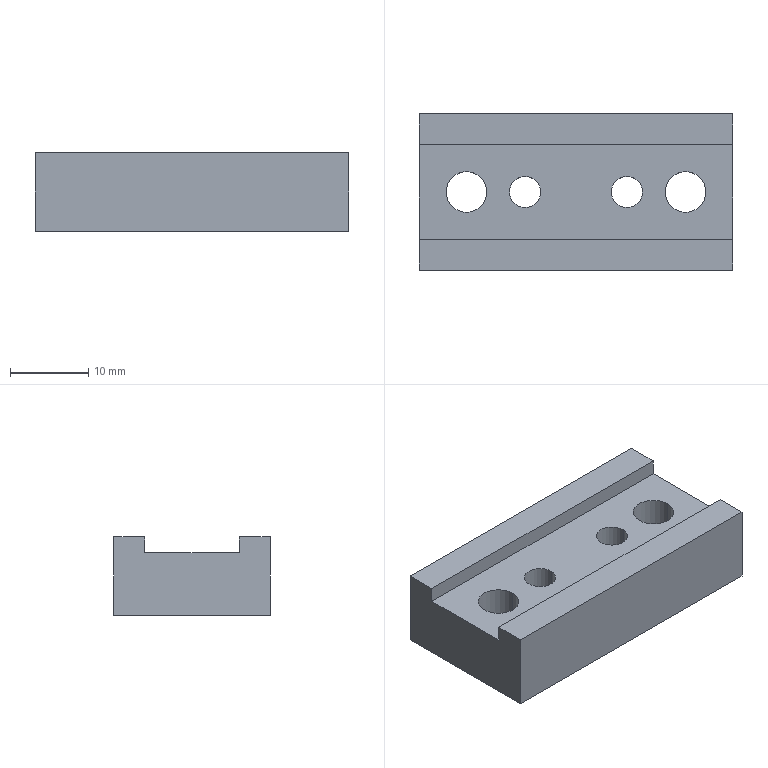Part | STEP file | PN_0031 | 1 solid | 18 faces | box 40 x 20 x 10 mm | volume 6491 mm3 | plane 10 | cylinder 8 | commonest cylinder face diameters 4 x4 5.2 x4
STEP:
#1=CARTESIAN_POINT('',(0.,0.,0.));
#2=DIRECTION('',(0.,0.,1.));
#3=DIRECTION('',(1.,0.,0.));
#4=AXIS2_PLACEMENT_3D('',#1,#2,#3);
#5=CARTESIAN_POINT('',(16.6,0.,0.));
#6=VERTEX_POINT('',#5);
#7=CARTESIAN_POINT('',(16.6,0.,8.));
#8=VERTEX_POINT('',#7);
#9=CARTESIAN_POINT('',(16.6,0.,-7.354));
#10=DIRECTION('',(0.,0.,1.));
#11=VECTOR('',#10,1.);
#12=LINE('',#9,#11);
#13=CARTESIAN_POINT('',(14.,0.,-7.354));
#14=DIRECTION('',(0.,0.,1.));
#15=DIRECTION('',(1.,0.,0.));
#16=AXIS2_PLACEMENT_3D('',#13,#14,#15);
#17=CYLINDRICAL_SURFACE('',#16,2.6);
#18=CARTESIAN_POINT('',(6.283,0.));
#19=DIRECTION('',(0.,1.));
#20=VECTOR('',#19,1.);
#21=LINE('',#18,#20);
#22=(GEOMETRIC_REPRESENTATION_CONTEXT(2)PARAMETRIC_REPRESENTATION_CONTEXT()REPRESENTATION_CONTEXT('',''));
#23=DEFINITIONAL_REPRESENTATION('',(#21),#22);
#24=PCURVE('',#17,#23);
#25=CARTESIAN_POINT('',(14.,0.,-7.354));
#26=DIRECTION('',(0.,0.,1.));
#27=DIRECTION('',(1.,0.,0.));
#28=AXIS2_PLACEMENT_3D('',#25,#26,#27);
#29=CYLINDRICAL_SURFACE('',#28,2.6);
#30=CARTESIAN_POINT('',(0.,0.));
#31=DIRECTION('',(0.,1.));
#32=VECTOR('',#31,1.);
#33=LINE('',#30,#32);
#34=(GEOMETRIC_REPRESENTATION_CONTEXT(2)PARAMETRIC_REPRESENTATION_CONTEXT()REPRESENTATION_CONTEXT('',''));
#35=DEFINITIONAL_REPRESENTATION('',(#33),#34);
#36=PCURVE('',#29,#35);
#37=SURFACE_CURVE('',#12,(#24,#36),.PCURVE_S1.);
#38=EDGE_CURVE('',#6,#8,#37,.T.);
#39=ORIENTED_EDGE('',*,*,#38,.T.);
#40=CARTESIAN_POINT('',(11.4,0.,8.));
#41=VERTEX_POINT('',#40);
#42=CARTESIAN_POINT('',(14.,0.,8.));
#43=DIRECTION('',(0.,0.,1.));
#44=DIRECTION('',(1.,0.,0.));
#45=AXIS2_PLACEMENT_3D('',#42,#43,#44);
#46=CIRCLE('',#45,2.6);
#47=CARTESIAN_POINT('',(0.,15.354));
#48=DIRECTION('',(1.,0.));
#49=VECTOR('',#48,1.);
#50=LINE('',#47,#49);
#51=(GEOMETRIC_REPRESENTATION_CONTEXT(2)PARAMETRIC_REPRESENTATION_CONTEXT()REPRESENTATION_CONTEXT('',''));
#52=DEFINITIONAL_REPRESENTATION('',(#50),#51);
#53=PCURVE('',#17,#52);
#54=CARTESIAN_POINT('',(0.,0.,8.));
#55=DIRECTION('',(0.,0.,-1.));
#56=DIRECTION('',(-1.,0.,0.));
#57=AXIS2_PLACEMENT_3D('',#54,#55,#56);
#58=PLANE('',#57);
#59=CARTESIAN_POINT('',(-16.6,0.));
#60=CARTESIAN_POINT('',(-16.6,4.503));
#61=CARTESIAN_POINT('',(-12.7,2.252));
#62=CARTESIAN_POINT('',(-8.8,0.));
#63=CARTESIAN_POINT('',(-12.7,-2.252));
#64=CARTESIAN_POINT('',(-16.6,-4.503));
#65=CARTESIAN_POINT('',(-16.6,0.));
#66=(BOUNDED_CURVE()B_SPLINE_CURVE(2,(#59,#60,#61,#62,#63,#64,#65),.UNSPECIFIED.,.T.,.F.)B_SPLINE_CURVE_WITH_KNOTS((1,2,2,2,2,1),(-2.094,0.,2.094,4.189,6.283,8.378),.UNSPECIFIED.)CURVE()GEOMETRIC_REPRESENTATION_ITEM()RATIONAL_B_SPLINE_CURVE((1.,0.5,1.,0.5,1.,0.5,1.))REPRESENTATION_ITEM(''));
#67=(GEOMETRIC_REPRESENTATION_CONTEXT(2)PARAMETRIC_REPRESENTATION_CONTEXT()REPRESENTATION_CONTEXT('',''));
#68=DEFINITIONAL_REPRESENTATION('',(#66),#67);
#69=PCURVE('',#58,#68);
#70=SURFACE_CURVE('',#46,(#53,#69),.PCURVE_S1.);
#71=EDGE_CURVE('',#41,#8,#70,.T.);
#72=ORIENTED_EDGE('',*,*,#71,.F.);
#73=CARTESIAN_POINT('',(11.4,0.,0.));
#74=VERTEX_POINT('',#73);
#75=CARTESIAN_POINT('',(11.4,0.,-7.354));
#76=DIRECTION('',(0.,0.,1.));
#77=VECTOR('',#76,1.);
#78=LINE('',#75,#77);
#79=CARTESIAN_POINT('',(3.142,0.));
#80=DIRECTION('',(0.,1.));
#81=VECTOR('',#80,1.);
#82=LINE('',#79,#81);
#83=(GEOMETRIC_REPRESENTATION_CONTEXT(2)PARAMETRIC_REPRESENTATION_CONTEXT()REPRESENTATION_CONTEXT('',''));
#84=DEFINITIONAL_REPRESENTATION('',(#82),#83);
#85=PCURVE('',#17,#84);
#86=CARTESIAN_POINT('',(3.142,0.));
#87=DIRECTION('',(0.,1.));
#88=VECTOR('',#87,1.);
#89=LINE('',#86,#88);
#90=(GEOMETRIC_REPRESENTATION_CONTEXT(2)PARAMETRIC_REPRESENTATION_CONTEXT()REPRESENTATION_CONTEXT('',''));
#91=DEFINITIONAL_REPRESENTATION('',(#89),#90);
#92=PCURVE('',#29,#91);
#93=SURFACE_CURVE('',#78,(#85,#92),.PCURVE_S1.);
#94=EDGE_CURVE('',#74,#41,#93,.T.);
#95=ORIENTED_EDGE('',*,*,#94,.F.);
#96=CARTESIAN_POINT('',(14.,0.,0.));
#97=DIRECTION('',(0.,0.,1.));
#98=DIRECTION('',(-1.,0.,0.));
#99=AXIS2_PLACEMENT_3D('',#96,#97,#98);
#100=CIRCLE('',#99,2.6);
#101=CARTESIAN_POINT('',(3.142,7.354));
#102=DIRECTION('',(1.,0.));
#103=VECTOR('',#102,1.);
#104=LINE('',#101,#103);
#105=(GEOMETRIC_REPRESENTATION_CONTEXT(2)PARAMETRIC_REPRESENTATION_CONTEXT()REPRESENTATION_CONTEXT('',''));
#106=DEFINITIONAL_REPRESENTATION('',(#104),#105);
#107=PCURVE('',#17,#106);
#108=CARTESIAN_POINT('',(0.,0.,0.));
#109=DIRECTION('',(0.,0.,-1.));
#110=DIRECTION('',(-1.,0.,0.));
#111=AXIS2_PLACEMENT_3D('',#108,#109,#110);
#112=PLANE('',#111);
#113=CARTESIAN_POINT('',(-11.4,0.));
#114=CARTESIAN_POINT('',(-11.4,-4.503));
#115=CARTESIAN_POINT('',(-15.3,-2.252));
#116=CARTESIAN_POINT('',(-19.2,0.));
#117=CARTESIAN_POINT('',(-15.3,2.252));
#118=CARTESIAN_POINT('',(-11.4,4.503));
#119=CARTESIAN_POINT('',(-11.4,0.));
#120=(BOUNDED_CURVE()B_SPLINE_CURVE(2,(#113,#114,#115,#116,#117,#118,#119),.UNSPECIFIED.,.T.,.F.)B_SPLINE_CURVE_WITH_KNOTS((1,2,2,2,2,1),(-2.094,0.,2.094,4.189,6.283,8.378),.UNSPECIFIED.)CURVE()GEOMETRIC_REPRESENTATION_ITEM()RATIONAL_B_SPLINE_CURVE((1.,0.5,1.,0.5,1.,0.5,1.))REPRESENTATION_ITEM(''));
#121=(GEOMETRIC_REPRESENTATION_CONTEXT(2)PARAMETRIC_REPRESENTATION_CONTEXT()REPRESENTATION_CONTEXT('',''));
#122=DEFINITIONAL_REPRESENTATION('',(#120),#121);
#123=PCURVE('',#112,#122);
#124=SURFACE_CURVE('',#100,(#107,#123),.PCURVE_S1.);
#125=EDGE_CURVE('',#74,#6,#124,.T.);
#126=ORIENTED_EDGE('',*,*,#125,.T.);
#127=EDGE_LOOP('',(#39,#72,#95,#126));
#128=FACE_BOUND('',#127,.F.);
#129=ADVANCED_FACE('',(#128),#17,.F.);
#130=CARTESIAN_POINT('',(-11.4,0.,0.));
#131=VERTEX_POINT('',#130);
#132=CARTESIAN_POINT('',(-11.4,0.,8.));
#133=VERTEX_POINT('',#132);
#134=CARTESIAN_POINT('',(-11.4,0.,-7.354));
#135=DIRECTION('',(0.,0.,1.));
#136=VECTOR('',#135,1.);
#137=LINE('',#134,#136);
#138=CARTESIAN_POINT('',(-14.,0.,-7.354));
#139=DIRECTION('',(0.,0.,1.));
#140=DIRECTION('',(1.,0.,0.));
#141=AXIS2_PLACEMENT_3D('',#138,#139,#140);
#142=CYLINDRICAL_SURFACE('',#141,2.6);
#143=CARTESIAN_POINT('',(6.283,0.));
#144=DIRECTION('',(0.,1.));
#145=VECTOR('',#144,1.);
#146=LINE('',#143,#145);
#147=(GEOMETRIC_REPRESENTATION_CONTEXT(2)PARAMETRIC_REPRESENTATION_CONTEXT()REPRESENTATION_CONTEXT('',''));
#148=DEFINITIONAL_REPRESENTATION('',(#146),#147);
#149=PCURVE('',#142,#148);
#150=CARTESIAN_POINT('',(-14.,0.,-7.354));
#151=DIRECTION('',(0.,0.,1.));
#152=DIRECTION('',(1.,0.,0.));
#153=AXIS2_PLACEMENT_3D('',#150,#151,#152);
#154=CYLINDRICAL_SURFACE('',#153,2.6);
#155=CARTESIAN_POINT('',(0.,0.));
#156=DIRECTION('',(0.,1.));
#157=VECTOR('',#156,1.);
#158=LINE('',#155,#157);
#159=(GEOMETRIC_REPRESENTATION_CONTEXT(2)PARAMETRIC_REPRESENTATION_CONTEXT()REPRESENTATION_CONTEXT('',''));
#160=DEFINITIONAL_REPRESENTATION('',(#158),#159);
#161=PCURVE('',#154,#160);
#162=SURFACE_CURVE('',#137,(#149,#161),.PCURVE_S1.);
#163=EDGE_CURVE('',#131,#133,#162,.T.);
#164=ORIENTED_EDGE('',*,*,#163,.T.);
#165=CARTESIAN_POINT('',(-16.6,0.,8.));
#166=VERTEX_POINT('',#165);
#167=CARTESIAN_POINT('',(-14.,0.,8.));
#168=DIRECTION('',(0.,0.,1.));
#169=DIRECTION('',(1.,0.,0.));
#170=AXIS2_PLACEMENT_3D('',#167,#168,#169);
#171=CIRCLE('',#170,2.6);
#172=CARTESIAN_POINT('',(0.,15.354));
#173=DIRECTION('',(1.,0.));
#174=VECTOR('',#173,1.);
#175=LINE('',#172,#174);
#176=(GEOMETRIC_REPRESENTATION_CONTEXT(2)PARAMETRIC_REPRESENTATION_CONTEXT()REPRESENTATION_CONTEXT('',''));
#177=DEFINITIONAL_REPRESENTATION('',(#175),#176);
#178=PCURVE('',#142,#177);
#179=CARTESIAN_POINT('',(11.4,0.));
#180=CARTESIAN_POINT('',(11.4,4.503));
#181=CARTESIAN_POINT('',(15.3,2.252));
#182=CARTESIAN_POINT('',(19.2,0.));
#183=CARTESIAN_POINT('',(15.3,-2.252));
#184=CARTESIAN_POINT('',(11.4,-4.503));
#185=CARTESIAN_POINT('',(11.4,0.));
#186=(BOUNDED_CURVE()B_SPLINE_CURVE(2,(#179,#180,#181,#182,#183,#184,#185),.UNSPECIFIED.,.T.,.F.)B_SPLINE_CURVE_WITH_KNOTS((1,2,2,2,2,1),(-2.094,0.,2.094,4.189,6.283,8.378),.UNSPECIFIED.)CURVE()GEOMETRIC_REPRESENTATION_ITEM()RATIONAL_B_SPLINE_CURVE((1.,0.5,1.,0.5,1.,0.5,1.))REPRESENTATION_ITEM(''));
#187=(GEOMETRIC_REPRESENTATION_CONTEXT(2)PARAMETRIC_REPRESENTATION_CONTEXT()REPRESENTATION_CONTEXT('',''));
#188=DEFINITIONAL_REPRESENTATION('',(#186),#187);
#189=PCURVE('',#58,#188);
#190=SURFACE_CURVE('',#171,(#178,#189),.PCURVE_S1.);
#191=EDGE_CURVE('',#166,#133,#190,.T.);
#192=ORIENTED_EDGE('',*,*,#191,.F.);
#193=CARTESIAN_POINT('',(-16.6,0.,0.));
#194=VERTEX_POINT('',#193);
#195=CARTESIAN_POINT('',(-16.6,0.,-7.354));
#196=DIRECTION('',(0.,0.,1.));
#197=VECTOR('',#196,1.);
#198=LINE('',#195,#197);
#199=CARTESIAN_POINT('',(3.142,0.));
#200=DIRECTION('',(0.,1.));
#201=VECTOR('',#200,1.);
#202=LINE('',#199,#201);
#203=(GEOMETRIC_REPRESENTATION_CONTEXT(2)PARAMETRIC_REPRESENTATION_CONTEXT()REPRESENTATION_CONTEXT('',''));
#204=DEFINITIONAL_REPRESENTATION('',(#202),#203);
#205=PCURVE('',#142,#204);
#206=CARTESIAN_POINT('',(3.142,0.));
#207=DIRECTION('',(0.,1.));
#208=VECTOR('',#207,1.);
#209=LINE('',#206,#208);
#210=(GEOMETRIC_REPRESENTATION_CONTEXT(2)PARAMETRIC_REPRESENTATION_CONTEXT()REPRESENTATION_CONTEXT('',''));
#211=DEFINITIONAL_REPRESENTATION('',(#209),#210);
#212=PCURVE('',#154,#211);
#213=SURFACE_CURVE('',#198,(#205,#212),.PCURVE_S1.);
#214=EDGE_CURVE('',#194,#166,#213,.T.);
#215=ORIENTED_EDGE('',*,*,#214,.F.);
#216=CARTESIAN_POINT('',(-14.,0.,0.));
#217=DIRECTION('',(0.,0.,1.));
#218=DIRECTION('',(-1.,0.,0.));
#219=AXIS2_PLACEMENT_3D('',#216,#217,#218);
#220=CIRCLE('',#219,2.6);
#221=CARTESIAN_POINT('',(3.142,7.354));
#222=DIRECTION('',(1.,0.));
#223=VECTOR('',#222,1.);
#224=LINE('',#221,#223);
#225=(GEOMETRIC_REPRESENTATION_CONTEXT(2)PARAMETRIC_REPRESENTATION_CONTEXT()REPRESENTATION_CONTEXT('',''));
#226=DEFINITIONAL_REPRESENTATION('',(#224),#225);
#227=PCURVE('',#142,#226);
#228=CARTESIAN_POINT('',(16.6,0.));
#229=CARTESIAN_POINT('',(16.6,-4.503));
#230=CARTESIAN_POINT('',(12.7,-2.252));
#231=CARTESIAN_POINT('',(8.8,0.));
#232=CARTESIAN_POINT('',(12.7,2.252));
#233=CARTESIAN_POINT('',(16.6,4.503));
#234=CARTESIAN_POINT('',(16.6,0.));
#235=(BOUNDED_CURVE()B_SPLINE_CURVE(2,(#228,#229,#230,#231,#232,#233,#234),.UNSPECIFIED.,.T.,.F.)B_SPLINE_CURVE_WITH_KNOTS((1,2,2,2,2,1),(-2.094,0.,2.094,4.189,6.283,8.378),.UNSPECIFIED.)CURVE()GEOMETRIC_REPRESENTATION_ITEM()RATIONAL_B_SPLINE_CURVE((1.,0.5,1.,0.5,1.,0.5,1.))REPRESENTATION_ITEM(''));
#236=(GEOMETRIC_REPRESENTATION_CONTEXT(2)PARAMETRIC_REPRESENTATION_CONTEXT()REPRESENTATION_CONTEXT('',''));
#237=DEFINITIONAL_REPRESENTATION('',(#235),#236);
#238=PCURVE('',#112,#237);
#239=SURFACE_CURVE('',#220,(#227,#238),.PCURVE_S1.);
#240=EDGE_CURVE('',#194,#131,#239,.T.);
#241=ORIENTED_EDGE('',*,*,#240,.T.);
#242=EDGE_LOOP('',(#164,#192,#215,#241));
#243=FACE_BOUND('',#242,.F.);
#244=ADVANCED_FACE('',(#243),#142,.F.);
#245=CARTESIAN_POINT('',(8.5,0.,0.));
#246=VERTEX_POINT('',#245);
#247=CARTESIAN_POINT('',(8.5,0.,8.));
#248=VERTEX_POINT('',#247);
#249=CARTESIAN_POINT('',(8.5,0.,-7.354));
#250=DIRECTION('',(0.,0.,1.));
#251=VECTOR('',#250,1.);
#252=LINE('',#249,#251);
#253=CARTESIAN_POINT('',(6.5,0.,-7.354));
#254=DIRECTION('',(0.,0.,1.));
#255=DIRECTION('',(1.,0.,0.));
#256=AXIS2_PLACEMENT_3D('',#253,#254,#255);
#257=CYLINDRICAL_SURFACE('',#256,2.);
#258=CARTESIAN_POINT('',(6.283,0.));
#259=DIRECTION('',(0.,1.));
#260=VECTOR('',#259,1.);
#261=LINE('',#258,#260);
#262=(GEOMETRIC_REPRESENTATION_CONTEXT(2)PARAMETRIC_REPRESENTATION_CONTEXT()REPRESENTATION_CONTEXT('',''));
#263=DEFINITIONAL_REPRESENTATION('',(#261),#262);
#264=PCURVE('',#257,#263);
#265=CARTESIAN_POINT('',(6.5,0.,-7.354));
#266=DIRECTION('',(0.,0.,1.));
#267=DIRECTION('',(1.,0.,0.));
#268=AXIS2_PLACEMENT_3D('',#265,#266,#267);
#269=CYLINDRICAL_SURFACE('',#268,2.);
#270=CARTESIAN_POINT('',(0.,0.));
#271=DIRECTION('',(0.,1.));
#272=VECTOR('',#271,1.);
#273=LINE('',#270,#272);
#274=(GEOMETRIC_REPRESENTATION_CONTEXT(2)PARAMETRIC_REPRESENTATION_CONTEXT()REPRESENTATION_CONTEXT('',''));
#275=DEFINITIONAL_REPRESENTATION('',(#273),#274);
#276=PCURVE('',#269,#275);
#277=SURFACE_CURVE('',#252,(#264,#276),.PCURVE_S1.);
#278=EDGE_CURVE('',#246,#248,#277,.T.);
#279=ORIENTED_EDGE('',*,*,#278,.T.);
#280=CARTESIAN_POINT('',(4.5,0.,8.));
#281=VERTEX_POINT('',#280);
#282=CARTESIAN_POINT('',(6.5,0.,8.));
#283=DIRECTION('',(0.,0.,1.));
#284=DIRECTION('',(1.,0.,0.));
#285=AXIS2_PLACEMENT_3D('',#282,#283,#284);
#286=CIRCLE('',#285,2.);
#287=CARTESIAN_POINT('',(0.,15.354));
#288=DIRECTION('',(1.,0.));
#289=VECTOR('',#288,1.);
#290=LINE('',#287,#289);
#291=(GEOMETRIC_REPRESENTATION_CONTEXT(2)PARAMETRIC_REPRESENTATION_CONTEXT()REPRESENTATION_CONTEXT('',''));
#292=DEFINITIONAL_REPRESENTATION('',(#290),#291);
#293=PCURVE('',#257,#292);
#294=CARTESIAN_POINT('',(-8.5,0.));
#295=CARTESIAN_POINT('',(-8.5,3.464));
#296=CARTESIAN_POINT('',(-5.5,1.732));
#297=CARTESIAN_POINT('',(-2.5,0.));
#298=CARTESIAN_POINT('',(-5.5,-1.732));
#299=CARTESIAN_POINT('',(-8.5,-3.464));
#300=CARTESIAN_POINT('',(-8.5,0.));
#301=(BOUNDED_CURVE()B_SPLINE_CURVE(2,(#294,#295,#296,#297,#298,#299,#300),.UNSPECIFIED.,.T.,.F.)B_SPLINE_CURVE_WITH_KNOTS((1,2,2,2,2,1),(-2.094,0.,2.094,4.189,6.283,8.378),.UNSPECIFIED.)CURVE()GEOMETRIC_REPRESENTATION_ITEM()RATIONAL_B_SPLINE_CURVE((1.,0.5,1.,0.5,1.,0.5,1.))REPRESENTATION_ITEM(''));
#302=(GEOMETRIC_REPRESENTATION_CONTEXT(2)PARAMETRIC_REPRESENTATION_CONTEXT()REPRESENTATION_CONTEXT('',''));
#303=DEFINITIONAL_REPRESENTATION('',(#301),#302);
#304=PCURVE('',#58,#303);
#305=SURFACE_CURVE('',#286,(#293,#304),.PCURVE_S1.);
#306=EDGE_CURVE('',#281,#248,#305,.T.);
#307=ORIENTED_EDGE('',*,*,#306,.F.);
#308=CARTESIAN_POINT('',(4.5,0.,0.));
#309=VERTEX_POINT('',#308);
#310=CARTESIAN_POINT('',(4.5,0.,-7.354));
#311=DIRECTION('',(0.,0.,1.));
#312=VECTOR('',#311,1.);
#313=LINE('',#310,#312);
#314=CARTESIAN_POINT('',(3.142,0.));
#315=DIRECTION('',(0.,1.));
#316=VECTOR('',#315,1.);
#317=LINE('',#314,#316);
#318=(GEOMETRIC_REPRESENTATION_CONTEXT(2)PARAMETRIC_REPRESENTATION_CONTEXT()REPRESENTATION_CONTEXT('',''));
#319=DEFINITIONAL_REPRESENTATION('',(#317),#318);
#320=PCURVE('',#257,#319);
#321=CARTESIAN_POINT('',(3.142,0.));
#322=DIRECTION('',(0.,1.));
#323=VECTOR('',#322,1.);
#324=LINE('',#321,#323);
#325=(GEOMETRIC_REPRESENTATION_CONTEXT(2)PARAMETRIC_REPRESENTATION_CONTEXT()REPRESENTATION_CONTEXT('',''));
#326=DEFINITIONAL_REPRESENTATION('',(#324),#325);
#327=PCURVE('',#269,#326);
#328=SURFACE_CURVE('',#313,(#320,#327),.PCURVE_S1.);
#329=EDGE_CURVE('',#309,#281,#328,.T.);
#330=ORIENTED_EDGE('',*,*,#329,.F.);
#331=CARTESIAN_POINT('',(6.5,0.,0.));
#332=DIRECTION('',(0.,0.,1.));
#333=DIRECTION('',(-1.,0.,0.));
#334=AXIS2_PLACEMENT_3D('',#331,#332,#333);
#335=CIRCLE('',#334,2.);
#336=CARTESIAN_POINT('',(3.142,7.354));
#337=DIRECTION('',(1.,0.));
#338=VECTOR('',#337,1.);
#339=LINE('',#336,#338);
#340=(GEOMETRIC_REPRESENTATION_CONTEXT(2)PARAMETRIC_REPRESENTATION_CONTEXT()REPRESENTATION_CONTEXT('',''));
#341=DEFINITIONAL_REPRESENTATION('',(#339),#340);
#342=PCURVE('',#257,#341);
#343=CARTESIAN_POINT('',(-4.5,0.));
#344=CARTESIAN_POINT('',(-4.5,-3.464));
#345=CARTESIAN_POINT('',(-7.5,-1.732));
#346=CARTESIAN_POINT('',(-10.5,0.));
#347=CARTESIAN_POINT('',(-7.5,1.732));
#348=CARTESIAN_POINT('',(-4.5,3.464));
#349=CARTESIAN_POINT('',(-4.5,0.));
#350=(BOUNDED_CURVE()B_SPLINE_CURVE(2,(#343,#344,#345,#346,#347,#348,#349),.UNSPECIFIED.,.T.,.F.)B_SPLINE_CURVE_WITH_KNOTS((1,2,2,2,2,1),(-2.094,0.,2.094,4.189,6.283,8.378),.UNSPECIFIED.)CURVE()GEOMETRIC_REPRESENTATION_ITEM()RATIONAL_B_SPLINE_CURVE((1.,0.5,1.,0.5,1.,0.5,1.))REPRESENTATION_ITEM(''));
#351=(GEOMETRIC_REPRESENTATION_CONTEXT(2)PARAMETRIC_REPRESENTATION_CONTEXT()REPRESENTATION_CONTEXT('',''));
#352=DEFINITIONAL_REPRESENTATION('',(#350),#351);
#353=PCURVE('',#112,#352);
#354=SURFACE_CURVE('',#335,(#342,#353),.PCURVE_S1.);
#355=EDGE_CURVE('',#309,#246,#354,.T.);
#356=ORIENTED_EDGE('',*,*,#355,.T.);
#357=EDGE_LOOP('',(#279,#307,#330,#356));
#358=FACE_BOUND('',#357,.F.);
#359=ADVANCED_FACE('',(#358),#257,.F.);
#360=CARTESIAN_POINT('',(-4.5,0.,0.));
#361=VERTEX_POINT('',#360);
#362=CARTESIAN_POINT('',(-4.5,0.,8.));
#363=VERTEX_POINT('',#362);
#364=CARTESIAN_POINT('',(-4.5,0.,-7.354));
#365=DIRECTION('',(0.,0.,1.));
#366=VECTOR('',#365,1.);
#367=LINE('',#364,#366);
#368=CARTESIAN_POINT('',(-6.5,0.,-7.354));
#369=DIRECTION('',(0.,0.,1.));
#370=DIRECTION('',(1.,0.,0.));
#371=AXIS2_PLACEMENT_3D('',#368,#369,#370);
#372=CYLINDRICAL_SURFACE('',#371,2.);
#373=CARTESIAN_POINT('',(6.283,0.));
#374=DIRECTION('',(0.,1.));
#375=VECTOR('',#374,1.);
#376=LINE('',#373,#375);
#377=(GEOMETRIC_REPRESENTATION_CONTEXT(2)PARAMETRIC_REPRESENTATION_CONTEXT()REPRESENTATION_CONTEXT('',''));
#378=DEFINITIONAL_REPRESENTATION('',(#376),#377);
#379=PCURVE('',#372,#378);
#380=CARTESIAN_POINT('',(-6.5,0.,-7.354));
#381=DIRECTION('',(0.,0.,1.));
#382=DIRECTION('',(1.,0.,0.));
#383=AXIS2_PLACEMENT_3D('',#380,#381,#382);
#384=CYLINDRICAL_SURFACE('',#383,2.);
#385=CARTESIAN_POINT('',(0.,0.));
#386=DIRECTION('',(0.,1.));
#387=VECTOR('',#386,1.);
#388=LINE('',#385,#387);
#389=(GEOMETRIC_REPRESENTATION_CONTEXT(2)PARAMETRIC_REPRESENTATION_CONTEXT()REPRESENTATION_CONTEXT('',''));
#390=DEFINITIONAL_REPRESENTATION('',(#388),#389);
#391=PCURVE('',#384,#390);
#392=SURFACE_CURVE('',#367,(#379,#391),.PCURVE_S1.);
#393=EDGE_CURVE('',#361,#363,#392,.T.);
#394=ORIENTED_EDGE('',*,*,#393,.T.);
#395=CARTESIAN_POINT('',(-8.5,0.,8.));
#396=VERTEX_POINT('',#395);
#397=CARTESIAN_POINT('',(-6.5,0.,8.));
#398=DIRECTION('',(0.,0.,1.));
#399=DIRECTION('',(1.,0.,0.));
#400=AXIS2_PLACEMENT_3D('',#397,#398,#399);
#401=CIRCLE('',#400,2.);
#402=CARTESIAN_POINT('',(0.,15.354));
#403=DIRECTION('',(1.,0.));
#404=VECTOR('',#403,1.);
#405=LINE('',#402,#404);
#406=(GEOMETRIC_REPRESENTATION_CONTEXT(2)PARAMETRIC_REPRESENTATION_CONTEXT()REPRESENTATION_CONTEXT('',''));
#407=DEFINITIONAL_REPRESENTATION('',(#405),#406);
#408=PCURVE('',#372,#407);
#409=CARTESIAN_POINT('',(4.5,0.));
#410=CARTESIAN_POINT('',(4.5,3.464));
#411=CARTESIAN_POINT('',(7.5,1.732));
#412=CARTESIAN_POINT('',(10.5,0.));
#413=CARTESIAN_POINT('',(7.5,-1.732));
#414=CARTESIAN_POINT('',(4.5,-3.464));
#415=CARTESIAN_POINT('',(4.5,0.));
#416=(BOUNDED_CURVE()B_SPLINE_CURVE(2,(#409,#410,#411,#412,#413,#414,#415),.UNSPECIFIED.,.T.,.F.)B_SPLINE_CURVE_WITH_KNOTS((1,2,2,2,2,1),(-2.094,0.,2.094,4.189,6.283,8.378),.UNSPECIFIED.)CURVE()GEOMETRIC_REPRESENTATION_ITEM()RATIONAL_B_SPLINE_CURVE((1.,0.5,1.,0.5,1.,0.5,1.))REPRESENTATION_ITEM(''));
#417=(GEOMETRIC_REPRESENTATION_CONTEXT(2)PARAMETRIC_REPRESENTATION_CONTEXT()REPRESENTATION_CONTEXT('',''));
#418=DEFINITIONAL_REPRESENTATION('',(#416),#417);
#419=PCURVE('',#58,#418);
#420=SURFACE_CURVE('',#401,(#408,#419),.PCURVE_S1.);
#421=EDGE_CURVE('',#396,#363,#420,.T.);
#422=ORIENTED_EDGE('',*,*,#421,.F.);
#423=CARTESIAN_POINT('',(-8.5,0.,0.));
#424=VERTEX_POINT('',#423);
#425=CARTESIAN_POINT('',(-8.5,0.,-7.354));
#426=DIRECTION('',(0.,0.,1.));
#427=VECTOR('',#426,1.);
#428=LINE('',#425,#427);
#429=CARTESIAN_POINT('',(3.142,0.));
#430=DIRECTION('',(0.,1.));
#431=VECTOR('',#430,1.);
#432=LINE('',#429,#431);
#433=(GEOMETRIC_REPRESENTATION_CONTEXT(2)PARAMETRIC_REPRESENTATION_CONTEXT()REPRESENTATION_CONTEXT('',''));
#434=DEFINITIONAL_REPRESENTATION('',(#432),#433);
#435=PCURVE('',#372,#434);
#436=CARTESIAN_POINT('',(3.142,0.));
#437=DIRECTION('',(0.,1.));
#438=VECTOR('',#437,1.);
#439=LINE('',#436,#438);
#440=(GEOMETRIC_REPRESENTATION_CONTEXT(2)PARAMETRIC_REPRESENTATION_CONTEXT()REPRESENTATION_CONTEXT('',''));
#441=DEFINITIONAL_REPRESENTATION('',(#439),#440);
#442=PCURVE('',#384,#441);
#443=SURFACE_CURVE('',#428,(#435,#442),.PCURVE_S1.);
#444=EDGE_CURVE('',#424,#396,#443,.T.);
#445=ORIENTED_EDGE('',*,*,#444,.F.);
#446=CARTESIAN_POINT('',(-6.5,0.,0.));
#447=DIRECTION('',(0.,0.,1.));
#448=DIRECTION('',(-1.,0.,0.));
#449=AXIS2_PLACEMENT_3D('',#446,#447,#448);
#450=CIRCLE('',#449,2.);
#451=CARTESIAN_POINT('',(3.142,7.354));
#452=DIRECTION('',(1.,0.));
#453=VECTOR('',#452,1.);
#454=LINE('',#451,#453);
#455=(GEOMETRIC_REPRESENTATION_CONTEXT(2)PARAMETRIC_REPRESENTATION_CONTEXT()REPRESENTATION_CONTEXT('',''));
#456=DEFINITIONAL_REPRESENTATION('',(#454),#455);
#457=PCURVE('',#372,#456);
#458=CARTESIAN_POINT('',(8.5,0.));
#459=CARTESIAN_POINT('',(8.5,-3.464));
#460=CARTESIAN_POINT('',(5.5,-1.732));
#461=CARTESIAN_POINT('',(2.5,0.));
#462=CARTESIAN_POINT('',(5.5,1.732));
#463=CARTESIAN_POINT('',(8.5,3.464));
#464=CARTESIAN_POINT('',(8.5,0.));
#465=(BOUNDED_CURVE()B_SPLINE_CURVE(2,(#458,#459,#460,#461,#462,#463,#464),.UNSPECIFIED.,.T.,.F.)B_SPLINE_CURVE_WITH_KNOTS((1,2,2,2,2,1),(-2.094,0.,2.094,4.189,6.283,8.378),.UNSPECIFIED.)CURVE()GEOMETRIC_REPRESENTATION_ITEM()RATIONAL_B_SPLINE_CURVE((1.,0.5,1.,0.5,1.,0.5,1.))REPRESENTATION_ITEM(''));
#466=(GEOMETRIC_REPRESENTATION_CONTEXT(2)PARAMETRIC_REPRESENTATION_CONTEXT()REPRESENTATION_CONTEXT('',''));
#467=DEFINITIONAL_REPRESENTATION('',(#465),#466);
#468=PCURVE('',#112,#467);
#469=SURFACE_CURVE('',#450,(#457,#468),.PCURVE_S1.);
#470=EDGE_CURVE('',#424,#361,#469,.T.);
#471=ORIENTED_EDGE('',*,*,#470,.T.);
#472=EDGE_LOOP('',(#394,#422,#445,#471));
#473=FACE_BOUND('',#472,.F.);
#474=ADVANCED_FACE('',(#473),#372,.F.);
#475=CARTESIAN_POINT('',(20.,-10.,10.));
#476=VERTEX_POINT('',#475);
#477=CARTESIAN_POINT('',(20.,-6.05,10.));
#478=VERTEX_POINT('',#477);
#479=CARTESIAN_POINT('',(20.,-10.,10.));
#480=DIRECTION('',(0.,1.,0.));
#481=VECTOR('',#480,1.);
#482=LINE('',#479,#481);
#483=CARTESIAN_POINT('',(0.,0.,10.));
#484=DIRECTION('',(0.,0.,-1.));
#485=DIRECTION('',(-1.,0.,0.));
#486=AXIS2_PLACEMENT_3D('',#483,#484,#485);
#487=PLANE('',#486);
#488=CARTESIAN_POINT('',(-20.,-10.));
#489=DIRECTION('',(0.,1.));
#490=VECTOR('',#489,1.);
#491=LINE('',#488,#490);
#492=(GEOMETRIC_REPRESENTATION_CONTEXT(2)PARAMETRIC_REPRESENTATION_CONTEXT()REPRESENTATION_CONTEXT('',''));
#493=DEFINITIONAL_REPRESENTATION('',(#491),#492);
#494=PCURVE('',#487,#493);
#495=CARTESIAN_POINT('',(20.,-10.,10.));
#496=DIRECTION('',(-1.,0.,0.));
#497=DIRECTION('',(0.,0.,1.));
#498=AXIS2_PLACEMENT_3D('',#495,#496,#497);
#499=PLANE('',#498);
#500=CARTESIAN_POINT('',(0.,0.));
#501=DIRECTION('',(0.,1.));
#502=VECTOR('',#501,1.);
#503=LINE('',#500,#502);
#504=(GEOMETRIC_REPRESENTATION_CONTEXT(2)PARAMETRIC_REPRESENTATION_CONTEXT()REPRESENTATION_CONTEXT('',''));
#505=DEFINITIONAL_REPRESENTATION('',(#503),#504);
#506=PCURVE('',#499,#505);
#507=SURFACE_CURVE('',#482,(#494,#506),.PCURVE_S1.);
#508=EDGE_CURVE('',#476,#478,#507,.T.);
#509=ORIENTED_EDGE('',*,*,#508,.T.);
#510=CARTESIAN_POINT('',(-20.,-6.05,10.));
#511=VERTEX_POINT('',#510);
#512=CARTESIAN_POINT('',(-20.,-6.05,10.));
#513=DIRECTION('',(1.,0.,0.));
#514=VECTOR('',#513,1.);
#515=LINE('',#512,#514);
#516=CARTESIAN_POINT('',(20.,-6.05));
#517=DIRECTION('',(-1.,0.));
#518=VECTOR('',#517,1.);
#519=LINE('',#516,#518);
#520=(GEOMETRIC_REPRESENTATION_CONTEXT(2)PARAMETRIC_REPRESENTATION_CONTEXT()REPRESENTATION_CONTEXT('',''));
#521=DEFINITIONAL_REPRESENTATION('',(#519),#520);
#522=PCURVE('',#487,#521);
#523=CARTESIAN_POINT('',(-20.,-6.05,8.));
#524=DIRECTION('',(0.,-1.,0.));
#525=DIRECTION('',(0.,0.,-1.));
#526=AXIS2_PLACEMENT_3D('',#523,#524,#525);
#527=PLANE('',#526);
#528=CARTESIAN_POINT('',(-2.,0.));
#529=DIRECTION('',(0.,1.));
#530=VECTOR('',#529,1.);
#531=LINE('',#528,#530);
#532=(GEOMETRIC_REPRESENTATION_CONTEXT(2)PARAMETRIC_REPRESENTATION_CONTEXT()REPRESENTATION_CONTEXT('',''));
#533=DEFINITIONAL_REPRESENTATION('',(#531),#532);
#534=PCURVE('',#527,#533);
#535=SURFACE_CURVE('',#515,(#522,#534),.PCURVE_S1.);
#536=EDGE_CURVE('',#511,#478,#535,.T.);
#537=ORIENTED_EDGE('',*,*,#536,.F.);
#538=CARTESIAN_POINT('',(-20.,-10.,10.));
#539=VERTEX_POINT('',#538);
#540=CARTESIAN_POINT('',(-20.,-10.,10.));
#541=DIRECTION('',(0.,-1.,0.));
#542=VECTOR('',#541,1.);
#543=LINE('',#540,#542);
#544=CARTESIAN_POINT('',(20.,-10.));
#545=DIRECTION('',(0.,-1.));
#546=VECTOR('',#545,1.);
#547=LINE('',#544,#546);
#548=(GEOMETRIC_REPRESENTATION_CONTEXT(2)PARAMETRIC_REPRESENTATION_CONTEXT()REPRESENTATION_CONTEXT('',''));
#549=DEFINITIONAL_REPRESENTATION('',(#547),#548);
#550=PCURVE('',#487,#549);
#551=CARTESIAN_POINT('',(-20.,-10.,10.));
#552=DIRECTION('',(1.,0.,0.));
#553=DIRECTION('',(0.,0.,-1.));
#554=AXIS2_PLACEMENT_3D('',#551,#552,#553);
#555=PLANE('',#554);
#556=CARTESIAN_POINT('',(0.,0.));
#557=DIRECTION('',(0.,-1.));
#558=VECTOR('',#557,1.);
#559=LINE('',#556,#558);
#560=(GEOMETRIC_REPRESENTATION_CONTEXT(2)PARAMETRIC_REPRESENTATION_CONTEXT()REPRESENTATION_CONTEXT('',''));
#561=DEFINITIONAL_REPRESENTATION('',(#559),#560);
#562=PCURVE('',#555,#561);
#563=SURFACE_CURVE('',#543,(#550,#562),.PCURVE_S1.);
#564=EDGE_CURVE('',#511,#539,#563,.T.);
#565=ORIENTED_EDGE('',*,*,#564,.T.);
#566=CARTESIAN_POINT('',(-20.,-10.,10.));
#567=DIRECTION('',(1.,0.,0.));
#568=VECTOR('',#567,1.);
#569=LINE('',#566,#568);
#570=CARTESIAN_POINT('',(20.,-10.));
#571=DIRECTION('',(-1.,0.));
#572=VECTOR('',#571,1.);
#573=LINE('',#570,#572);
#574=(GEOMETRIC_REPRESENTATION_CONTEXT(2)PARAMETRIC_REPRESENTATION_CONTEXT()REPRESENTATION_CONTEXT('',''));
#575=DEFINITIONAL_REPRESENTATION('',(#573),#574);
#576=PCURVE('',#487,#575);
#577=CARTESIAN_POINT('',(-20.,-10.,10.));
#578=DIRECTION('',(0.,1.,0.));
#579=DIRECTION('',(0.,0.,1.));
#580=AXIS2_PLACEMENT_3D('',#577,#578,#579);
#581=PLANE('',#580);
#582=CARTESIAN_POINT('',(0.,0.));
#583=DIRECTION('',(0.,1.));
#584=VECTOR('',#583,1.);
#585=LINE('',#582,#584);
#586=(GEOMETRIC_REPRESENTATION_CONTEXT(2)PARAMETRIC_REPRESENTATION_CONTEXT()REPRESENTATION_CONTEXT('',''));
#587=DEFINITIONAL_REPRESENTATION('',(#585),#586);
#588=PCURVE('',#581,#587);
#589=SURFACE_CURVE('',#569,(#576,#588),.PCURVE_S1.);
#590=EDGE_CURVE('',#539,#476,#589,.T.);
#591=ORIENTED_EDGE('',*,*,#590,.T.);
#592=EDGE_LOOP('',(#509,#537,#565,#591));
#593=FACE_BOUND('',#592,.T.);
#594=ADVANCED_FACE('',(#593),#487,.F.);
#595=CARTESIAN_POINT('',(20.,-6.05,8.));
#596=VERTEX_POINT('',#595);
#597=CARTESIAN_POINT('',(20.,6.05,8.));
#598=VERTEX_POINT('',#597);
#599=CARTESIAN_POINT('',(20.,-6.05,8.));
#600=DIRECTION('',(0.,1.,0.));
#601=VECTOR('',#600,1.);
#602=LINE('',#599,#601);
#603=CARTESIAN_POINT('',(-2.,3.95));
#604=DIRECTION('',(0.,1.));
#605=VECTOR('',#604,1.);
#606=LINE('',#603,#605);
#607=(GEOMETRIC_REPRESENTATION_CONTEXT(2)PARAMETRIC_REPRESENTATION_CONTEXT()REPRESENTATION_CONTEXT('',''));
#608=DEFINITIONAL_REPRESENTATION('',(#606),#607);
#609=PCURVE('',#499,#608);
#610=CARTESIAN_POINT('',(-20.,-6.05));
#611=DIRECTION('',(0.,1.));
#612=VECTOR('',#611,1.);
#613=LINE('',#610,#612);
#614=(GEOMETRIC_REPRESENTATION_CONTEXT(2)PARAMETRIC_REPRESENTATION_CONTEXT()REPRESENTATION_CONTEXT('',''));
#615=DEFINITIONAL_REPRESENTATION('',(#613),#614);
#616=PCURVE('',#58,#615);
#617=SURFACE_CURVE('',#602,(#609,#616),.PCURVE_S1.);
#618=EDGE_CURVE('',#596,#598,#617,.T.);
#619=ORIENTED_EDGE('',*,*,#618,.F.);
#620=CARTESIAN_POINT('',(20.,-6.05,8.));
#621=DIRECTION('',(0.,0.,1.));
#622=VECTOR('',#621,1.);
#623=LINE('',#620,#622);
#624=CARTESIAN_POINT('',(-2.,3.95));
#625=DIRECTION('',(1.,0.));
#626=VECTOR('',#625,1.);
#627=LINE('',#624,#626);
#628=(GEOMETRIC_REPRESENTATION_CONTEXT(2)PARAMETRIC_REPRESENTATION_CONTEXT()REPRESENTATION_CONTEXT('',''));
#629=DEFINITIONAL_REPRESENTATION('',(#627),#628);
#630=PCURVE('',#499,#629);
#631=CARTESIAN_POINT('',(0.,40.));
#632=DIRECTION('',(-1.,0.));
#633=VECTOR('',#632,1.);
#634=LINE('',#631,#633);
#635=(GEOMETRIC_REPRESENTATION_CONTEXT(2)PARAMETRIC_REPRESENTATION_CONTEXT()REPRESENTATION_CONTEXT('',''));
#636=DEFINITIONAL_REPRESENTATION('',(#634),#635);
#637=PCURVE('',#527,#636);
#638=SURFACE_CURVE('',#623,(#630,#637),.PCURVE_S1.);
#639=EDGE_CURVE('',#596,#478,#638,.T.);
#640=ORIENTED_EDGE('',*,*,#639,.T.);
#641=ORIENTED_EDGE('',*,*,#508,.F.);
#642=CARTESIAN_POINT('',(20.,-10.,0.));
#643=VERTEX_POINT('',#642);
#644=CARTESIAN_POINT('',(20.,-10.,10.));
#645=DIRECTION('',(0.,0.,-1.));
#646=VECTOR('',#645,1.);
#647=LINE('',#644,#646);
#648=CARTESIAN_POINT('',(0.,0.));
#649=DIRECTION('',(-1.,0.));
#650=VECTOR('',#649,1.);
#651=LINE('',#648,#650);
#652=(GEOMETRIC_REPRESENTATION_CONTEXT(2)PARAMETRIC_REPRESENTATION_CONTEXT()REPRESENTATION_CONTEXT('',''));
#653=DEFINITIONAL_REPRESENTATION('',(#651),#652);
#654=PCURVE('',#499,#653);
#655=CARTESIAN_POINT('',(0.,40.));
#656=DIRECTION('',(-1.,0.));
#657=VECTOR('',#656,1.);
#658=LINE('',#655,#657);
#659=(GEOMETRIC_REPRESENTATION_CONTEXT(2)PARAMETRIC_REPRESENTATION_CONTEXT()REPRESENTATION_CONTEXT('',''));
#660=DEFINITIONAL_REPRESENTATION('',(#658),#659);
#661=PCURVE('',#581,#660);
#662=SURFACE_CURVE('',#647,(#654,#661),.PCURVE_S1.);
#663=EDGE_CURVE('',#476,#643,#662,.T.);
#664=ORIENTED_EDGE('',*,*,#663,.T.);
#665=CARTESIAN_POINT('',(20.,10.,0.));
#666=VERTEX_POINT('',#665);
#667=CARTESIAN_POINT('',(20.,-10.,0.));
#668=DIRECTION('',(0.,1.,0.));
#669=VECTOR('',#668,1.);
#670=LINE('',#667,#669);
#671=CARTESIAN_POINT('',(-10.,0.));
#672=DIRECTION('',(0.,1.));
#673=VECTOR('',#672,1.);
#674=LINE('',#671,#673);
#675=(GEOMETRIC_REPRESENTATION_CONTEXT(2)PARAMETRIC_REPRESENTATION_CONTEXT()REPRESENTATION_CONTEXT('',''));
#676=DEFINITIONAL_REPRESENTATION('',(#674),#675);
#677=PCURVE('',#499,#676);
#678=CARTESIAN_POINT('',(-20.,-10.));
#679=DIRECTION('',(0.,1.));
#680=VECTOR('',#679,1.);
#681=LINE('',#678,#680);
#682=(GEOMETRIC_REPRESENTATION_CONTEXT(2)PARAMETRIC_REPRESENTATION_CONTEXT()REPRESENTATION_CONTEXT('',''));
#683=DEFINITIONAL_REPRESENTATION('',(#681),#682);
#684=PCURVE('',#112,#683);
#685=SURFACE_CURVE('',#670,(#677,#684),.PCURVE_S1.);
#686=EDGE_CURVE('',#643,#666,#685,.T.);
#687=ORIENTED_EDGE('',*,*,#686,.T.);
#688=CARTESIAN_POINT('',(20.,10.,10.));
#689=VERTEX_POINT('',#688);
#690=CARTESIAN_POINT('',(20.,10.,10.));
#691=DIRECTION('',(0.,0.,-1.));
#692=VECTOR('',#691,1.);
#693=LINE('',#690,#692);
#694=CARTESIAN_POINT('',(0.,20.));
#695=DIRECTION('',(-1.,0.));
#696=VECTOR('',#695,1.);
#697=LINE('',#694,#696);
#698=(GEOMETRIC_REPRESENTATION_CONTEXT(2)PARAMETRIC_REPRESENTATION_CONTEXT()REPRESENTATION_CONTEXT('',''));
#699=DEFINITIONAL_REPRESENTATION('',(#697),#698);
#700=PCURVE('',#499,#699);
#701=CARTESIAN_POINT('',(-20.,10.,10.));
#702=DIRECTION('',(0.,-1.,0.));
#703=DIRECTION('',(0.,0.,-1.));
#704=AXIS2_PLACEMENT_3D('',#701,#702,#703);
#705=PLANE('',#704);
#706=CARTESIAN_POINT('',(0.,40.));
#707=DIRECTION('',(1.,0.));
#708=VECTOR('',#707,1.);
#709=LINE('',#706,#708);
#710=(GEOMETRIC_REPRESENTATION_CONTEXT(2)PARAMETRIC_REPRESENTATION_CONTEXT()REPRESENTATION_CONTEXT('',''));
#711=DEFINITIONAL_REPRESENTATION('',(#709),#710);
#712=PCURVE('',#705,#711);
#713=SURFACE_CURVE('',#693,(#700,#712),.PCURVE_S1.);
#714=EDGE_CURVE('',#689,#666,#713,.T.);
#715=ORIENTED_EDGE('',*,*,#714,.F.);
#716=CARTESIAN_POINT('',(20.,6.05,10.));
#717=VERTEX_POINT('',#716);
#718=CARTESIAN_POINT('',(20.,-10.,10.));
#719=DIRECTION('',(0.,1.,0.));
#720=VECTOR('',#719,1.);
#721=LINE('',#718,#720);
#722=CARTESIAN_POINT('',(0.,0.));
#723=DIRECTION('',(0.,1.));
#724=VECTOR('',#723,1.);
#725=LINE('',#722,#724);
#726=(GEOMETRIC_REPRESENTATION_CONTEXT(2)PARAMETRIC_REPRESENTATION_CONTEXT()REPRESENTATION_CONTEXT('',''));
#727=DEFINITIONAL_REPRESENTATION('',(#725),#726);
#728=PCURVE('',#499,#727);
#729=CARTESIAN_POINT('',(0.,0.,10.));
#730=DIRECTION('',(0.,0.,-1.));
#731=DIRECTION('',(-1.,0.,0.));
#732=AXIS2_PLACEMENT_3D('',#729,#730,#731);
#733=PLANE('',#732);
#734=CARTESIAN_POINT('',(-20.,-10.));
#735=DIRECTION('',(0.,1.));
#736=VECTOR('',#735,1.);
#737=LINE('',#734,#736);
#738=(GEOMETRIC_REPRESENTATION_CONTEXT(2)PARAMETRIC_REPRESENTATION_CONTEXT()REPRESENTATION_CONTEXT('',''));
#739=DEFINITIONAL_REPRESENTATION('',(#737),#738);
#740=PCURVE('',#733,#739);
#741=SURFACE_CURVE('',#721,(#728,#740),.PCURVE_S1.);
#742=EDGE_CURVE('',#717,#689,#741,.T.);
#743=ORIENTED_EDGE('',*,*,#742,.F.);
#744=CARTESIAN_POINT('',(20.,6.05,8.));
#745=DIRECTION('',(0.,0.,1.));
#746=VECTOR('',#745,1.);
#747=LINE('',#744,#746);
#748=CARTESIAN_POINT('',(-2.,16.05));
#749=DIRECTION('',(1.,0.));
#750=VECTOR('',#749,1.);
#751=LINE('',#748,#750);
#752=(GEOMETRIC_REPRESENTATION_CONTEXT(2)PARAMETRIC_REPRESENTATION_CONTEXT()REPRESENTATION_CONTEXT('',''));
#753=DEFINITIONAL_REPRESENTATION('',(#751),#752);
#754=PCURVE('',#499,#753);
#755=CARTESIAN_POINT('',(-20.,6.05,8.));
#756=DIRECTION('',(0.,1.,0.));
#757=DIRECTION('',(0.,0.,1.));
#758=AXIS2_PLACEMENT_3D('',#755,#756,#757);
#759=PLANE('',#758);
#760=CARTESIAN_POINT('',(0.,40.));
#761=DIRECTION('',(1.,0.));
#762=VECTOR('',#761,1.);
#763=LINE('',#760,#762);
#764=(GEOMETRIC_REPRESENTATION_CONTEXT(2)PARAMETRIC_REPRESENTATION_CONTEXT()REPRESENTATION_CONTEXT('',''));
#765=DEFINITIONAL_REPRESENTATION('',(#763),#764);
#766=PCURVE('',#759,#765);
#767=SURFACE_CURVE('',#747,(#754,#766),.PCURVE_S1.);
#768=EDGE_CURVE('',#598,#717,#767,.T.);
#769=ORIENTED_EDGE('',*,*,#768,.F.);
#770=EDGE_LOOP('',(#619,#640,#641,#664,#687,#715,#743,#769));
#771=FACE_BOUND('',#770,.T.);
#772=ADVANCED_FACE('',(#771),#499,.F.);
#773=CARTESIAN_POINT('',(-20.,10.,0.));
#774=VERTEX_POINT('',#773);
#775=CARTESIAN_POINT('',(-20.,10.,0.));
#776=DIRECTION('',(-1.,0.,0.));
#777=VECTOR('',#776,1.);
#778=LINE('',#775,#777);
#779=CARTESIAN_POINT('',(10.,0.));
#780=DIRECTION('',(0.,-1.));
#781=VECTOR('',#780,1.);
#782=LINE('',#779,#781);
#783=(GEOMETRIC_REPRESENTATION_CONTEXT(2)PARAMETRIC_REPRESENTATION_CONTEXT()REPRESENTATION_CONTEXT('',''));
#784=DEFINITIONAL_REPRESENTATION('',(#782),#783);
#785=PCURVE('',#705,#784);
#786=CARTESIAN_POINT('',(20.,10.));
#787=DIRECTION('',(1.,0.));
#788=VECTOR('',#787,1.);
#789=LINE('',#786,#788);
#790=(GEOMETRIC_REPRESENTATION_CONTEXT(2)PARAMETRIC_REPRESENTATION_CONTEXT()REPRESENTATION_CONTEXT('',''));
#791=DEFINITIONAL_REPRESENTATION('',(#789),#790);
#792=PCURVE('',#112,#791);
#793=SURFACE_CURVE('',#778,(#785,#792),.PCURVE_S1.);
#794=EDGE_CURVE('',#666,#774,#793,.T.);
#795=ORIENTED_EDGE('',*,*,#794,.T.);
#796=CARTESIAN_POINT('',(-20.,10.,10.));
#797=VERTEX_POINT('',#796);
#798=CARTESIAN_POINT('',(-20.,10.,10.));
#799=DIRECTION('',(0.,0.,-1.));
#800=VECTOR('',#799,1.);
#801=LINE('',#798,#800);
#802=CARTESIAN_POINT('',(0.,0.));
#803=DIRECTION('',(1.,0.));
#804=VECTOR('',#803,1.);
#805=LINE('',#802,#804);
#806=(GEOMETRIC_REPRESENTATION_CONTEXT(2)PARAMETRIC_REPRESENTATION_CONTEXT()REPRESENTATION_CONTEXT('',''));
#807=DEFINITIONAL_REPRESENTATION('',(#805),#806);
#808=PCURVE('',#705,#807);
#809=CARTESIAN_POINT('',(0.,20.));
#810=DIRECTION('',(1.,0.));
#811=VECTOR('',#810,1.);
#812=LINE('',#809,#811);
#813=(GEOMETRIC_REPRESENTATION_CONTEXT(2)PARAMETRIC_REPRESENTATION_CONTEXT()REPRESENTATION_CONTEXT('',''));
#814=DEFINITIONAL_REPRESENTATION('',(#812),#813);
#815=PCURVE('',#555,#814);
#816=SURFACE_CURVE('',#801,(#808,#815),.PCURVE_S1.);
#817=EDGE_CURVE('',#797,#774,#816,.T.);
#818=ORIENTED_EDGE('',*,*,#817,.F.);
#819=CARTESIAN_POINT('',(-20.,10.,10.));
#820=DIRECTION('',(-1.,0.,0.));
#821=VECTOR('',#820,1.);
#822=LINE('',#819,#821);
#823=CARTESIAN_POINT('',(0.,0.));
#824=DIRECTION('',(0.,-1.));
#825=VECTOR('',#824,1.);
#826=LINE('',#823,#825);
#827=(GEOMETRIC_REPRESENTATION_CONTEXT(2)PARAMETRIC_REPRESENTATION_CONTEXT()REPRESENTATION_CONTEXT('',''));
#828=DEFINITIONAL_REPRESENTATION('',(#826),#827);
#829=PCURVE('',#705,#828);
#830=CARTESIAN_POINT('',(20.,10.));
#831=DIRECTION('',(1.,0.));
#832=VECTOR('',#831,1.);
#833=LINE('',#830,#832);
#834=(GEOMETRIC_REPRESENTATION_CONTEXT(2)PARAMETRIC_REPRESENTATION_CONTEXT()REPRESENTATION_CONTEXT('',''));
#835=DEFINITIONAL_REPRESENTATION('',(#833),#834);
#836=PCURVE('',#733,#835);
#837=SURFACE_CURVE('',#822,(#829,#836),.PCURVE_S1.);
#838=EDGE_CURVE('',#689,#797,#837,.T.);
#839=ORIENTED_EDGE('',*,*,#838,.F.);
#840=ORIENTED_EDGE('',*,*,#714,.T.);
#841=EDGE_LOOP('',(#795,#818,#839,#840));
#842=FACE_BOUND('',#841,.T.);
#843=ADVANCED_FACE('',(#842),#705,.F.);
#844=ORIENTED_EDGE('',*,*,#564,.F.);
#845=CARTESIAN_POINT('',(-20.,-6.05,8.));
#846=VERTEX_POINT('',#845);
#847=CARTESIAN_POINT('',(-20.,-6.05,8.));
#848=DIRECTION('',(0.,0.,1.));
#849=VECTOR('',#848,1.);
#850=LINE('',#847,#849);
#851=CARTESIAN_POINT('',(2.,3.95));
#852=DIRECTION('',(-1.,0.));
#853=VECTOR('',#852,1.);
#854=LINE('',#851,#853);
#855=(GEOMETRIC_REPRESENTATION_CONTEXT(2)PARAMETRIC_REPRESENTATION_CONTEXT()REPRESENTATION_CONTEXT('',''));
#856=DEFINITIONAL_REPRESENTATION('',(#854),#855);
#857=PCURVE('',#555,#856);
#858=CARTESIAN_POINT('',(0.,0.));
#859=DIRECTION('',(-1.,0.));
#860=VECTOR('',#859,1.);
#861=LINE('',#858,#860);
#862=(GEOMETRIC_REPRESENTATION_CONTEXT(2)PARAMETRIC_REPRESENTATION_CONTEXT()REPRESENTATION_CONTEXT('',''));
#863=DEFINITIONAL_REPRESENTATION('',(#861),#862);
#864=PCURVE('',#527,#863);
#865=SURFACE_CURVE('',#850,(#857,#864),.PCURVE_S1.);
#866=EDGE_CURVE('',#846,#511,#865,.T.);
#867=ORIENTED_EDGE('',*,*,#866,.F.);
#868=CARTESIAN_POINT('',(-20.,6.05,8.));
#869=VERTEX_POINT('',#868);
#870=CARTESIAN_POINT('',(-20.,-6.05,8.));
#871=DIRECTION('',(0.,-1.,0.));
#872=VECTOR('',#871,1.);
#873=LINE('',#870,#872);
#874=CARTESIAN_POINT('',(2.,3.95));
#875=DIRECTION('',(0.,-1.));
#876=VECTOR('',#875,1.);
#877=LINE('',#874,#876);
#878=(GEOMETRIC_REPRESENTATION_CONTEXT(2)PARAMETRIC_REPRESENTATION_CONTEXT()REPRESENTATION_CONTEXT('',''));
#879=DEFINITIONAL_REPRESENTATION('',(#877),#878);
#880=PCURVE('',#555,#879);
#881=CARTESIAN_POINT('',(20.,-6.05));
#882=DIRECTION('',(0.,-1.));
#883=VECTOR('',#882,1.);
#884=LINE('',#881,#883);
#885=(GEOMETRIC_REPRESENTATION_CONTEXT(2)PARAMETRIC_REPRESENTATION_CONTEXT()REPRESENTATION_CONTEXT('',''));
#886=DEFINITIONAL_REPRESENTATION('',(#884),#885);
#887=PCURVE('',#58,#886);
#888=SURFACE_CURVE('',#873,(#880,#887),.PCURVE_S1.);
#889=EDGE_CURVE('',#869,#846,#888,.T.);
#890=ORIENTED_EDGE('',*,*,#889,.F.);
#891=CARTESIAN_POINT('',(-20.,6.05,10.));
#892=VERTEX_POINT('',#891);
#893=CARTESIAN_POINT('',(-20.,6.05,8.));
#894=DIRECTION('',(0.,0.,1.));
#895=VECTOR('',#894,1.);
#896=LINE('',#893,#895);
#897=CARTESIAN_POINT('',(2.,16.05));
#898=DIRECTION('',(-1.,0.));
#899=VECTOR('',#898,1.);
#900=LINE('',#897,#899);
#901=(GEOMETRIC_REPRESENTATION_CONTEXT(2)PARAMETRIC_REPRESENTATION_CONTEXT()REPRESENTATION_CONTEXT('',''));
#902=DEFINITIONAL_REPRESENTATION('',(#900),#901);
#903=PCURVE('',#555,#902);
#904=CARTESIAN_POINT('',(0.,0.));
#905=DIRECTION('',(1.,0.));
#906=VECTOR('',#905,1.);
#907=LINE('',#904,#906);
#908=(GEOMETRIC_REPRESENTATION_CONTEXT(2)PARAMETRIC_REPRESENTATION_CONTEXT()REPRESENTATION_CONTEXT('',''));
#909=DEFINITIONAL_REPRESENTATION('',(#907),#908);
#910=PCURVE('',#759,#909);
#911=SURFACE_CURVE('',#896,(#903,#910),.PCURVE_S1.);
#912=EDGE_CURVE('',#869,#892,#911,.T.);
#913=ORIENTED_EDGE('',*,*,#912,.T.);
#914=CARTESIAN_POINT('',(-20.,-10.,10.));
#915=DIRECTION('',(0.,-1.,0.));
#916=VECTOR('',#915,1.);
#917=LINE('',#914,#916);
#918=CARTESIAN_POINT('',(0.,0.));
#919=DIRECTION('',(0.,-1.));
#920=VECTOR('',#919,1.);
#921=LINE('',#918,#920);
#922=(GEOMETRIC_REPRESENTATION_CONTEXT(2)PARAMETRIC_REPRESENTATION_CONTEXT()REPRESENTATION_CONTEXT('',''));
#923=DEFINITIONAL_REPRESENTATION('',(#921),#922);
#924=PCURVE('',#555,#923);
#925=CARTESIAN_POINT('',(20.,-10.));
#926=DIRECTION('',(0.,-1.));
#927=VECTOR('',#926,1.);
#928=LINE('',#925,#927);
#929=(GEOMETRIC_REPRESENTATION_CONTEXT(2)PARAMETRIC_REPRESENTATION_CONTEXT()REPRESENTATION_CONTEXT('',''));
#930=DEFINITIONAL_REPRESENTATION('',(#928),#929);
#931=PCURVE('',#733,#930);
#932=SURFACE_CURVE('',#917,(#924,#931),.PCURVE_S1.);
#933=EDGE_CURVE('',#797,#892,#932,.T.);
#934=ORIENTED_EDGE('',*,*,#933,.F.);
#935=ORIENTED_EDGE('',*,*,#817,.T.);
#936=CARTESIAN_POINT('',(-20.,-10.,0.));
#937=VERTEX_POINT('',#936);
#938=CARTESIAN_POINT('',(-20.,-10.,0.));
#939=DIRECTION('',(0.,-1.,0.));
#940=VECTOR('',#939,1.);
#941=LINE('',#938,#940);
#942=CARTESIAN_POINT('',(10.,0.));
#943=DIRECTION('',(0.,-1.));
#944=VECTOR('',#943,1.);
#945=LINE('',#942,#944);
#946=(GEOMETRIC_REPRESENTATION_CONTEXT(2)PARAMETRIC_REPRESENTATION_CONTEXT()REPRESENTATION_CONTEXT('',''));
#947=DEFINITIONAL_REPRESENTATION('',(#945),#946);
#948=PCURVE('',#555,#947);
#949=CARTESIAN_POINT('',(20.,-10.));
#950=DIRECTION('',(0.,-1.));
#951=VECTOR('',#950,1.);
#952=LINE('',#949,#951);
#953=(GEOMETRIC_REPRESENTATION_CONTEXT(2)PARAMETRIC_REPRESENTATION_CONTEXT()REPRESENTATION_CONTEXT('',''));
#954=DEFINITIONAL_REPRESENTATION('',(#952),#953);
#955=PCURVE('',#112,#954);
#956=SURFACE_CURVE('',#941,(#948,#955),.PCURVE_S1.);
#957=EDGE_CURVE('',#774,#937,#956,.T.);
#958=ORIENTED_EDGE('',*,*,#957,.T.);
#959=CARTESIAN_POINT('',(-20.,-10.,10.));
#960=DIRECTION('',(0.,0.,-1.));
#961=VECTOR('',#960,1.);
#962=LINE('',#959,#961);
#963=CARTESIAN_POINT('',(0.,0.));
#964=DIRECTION('',(1.,0.));
#965=VECTOR('',#964,1.);
#966=LINE('',#963,#965);
#967=(GEOMETRIC_REPRESENTATION_CONTEXT(2)PARAMETRIC_REPRESENTATION_CONTEXT()REPRESENTATION_CONTEXT('',''));
#968=DEFINITIONAL_REPRESENTATION('',(#966),#967);
#969=PCURVE('',#555,#968);
#970=CARTESIAN_POINT('',(0.,0.));
#971=DIRECTION('',(-1.,0.));
#972=VECTOR('',#971,1.);
#973=LINE('',#970,#972);
#974=(GEOMETRIC_REPRESENTATION_CONTEXT(2)PARAMETRIC_REPRESENTATION_CONTEXT()REPRESENTATION_CONTEXT('',''));
#975=DEFINITIONAL_REPRESENTATION('',(#973),#974);
#976=PCURVE('',#581,#975);
#977=SURFACE_CURVE('',#962,(#969,#976),.PCURVE_S1.);
#978=EDGE_CURVE('',#539,#937,#977,.T.);
#979=ORIENTED_EDGE('',*,*,#978,.F.);
#980=EDGE_LOOP('',(#844,#867,#890,#913,#934,#935,#958,#979));
#981=FACE_BOUND('',#980,.T.);
#982=ADVANCED_FACE('',(#981),#555,.F.);
#983=CARTESIAN_POINT('',(-20.,-10.,0.));
#984=DIRECTION('',(1.,0.,0.));
#985=VECTOR('',#984,1.);
#986=LINE('',#983,#985);
#987=CARTESIAN_POINT('',(-10.,0.));
#988=DIRECTION('',(0.,1.));
#989=VECTOR('',#988,1.);
#990=LINE('',#987,#989);
#991=(GEOMETRIC_REPRESENTATION_CONTEXT(2)PARAMETRIC_REPRESENTATION_CONTEXT()REPRESENTATION_CONTEXT('',''));
#992=DEFINITIONAL_REPRESENTATION('',(#990),#991);
#993=PCURVE('',#581,#992);
#994=CARTESIAN_POINT('',(20.,-10.));
#995=DIRECTION('',(-1.,0.));
#996=VECTOR('',#995,1.);
#997=LINE('',#994,#996);
#998=(GEOMETRIC_REPRESENTATION_CONTEXT(2)PARAMETRIC_REPRESENTATION_CONTEXT()REPRESENTATION_CONTEXT('',''));
#999=DEFINITIONAL_REPRESENTATION('',(#997),#998);
#1000=PCURVE('',#112,#999);
#1001=SURFACE_CURVE('',#986,(#993,#1000),.PCURVE_S1.);
#1002=EDGE_CURVE('',#937,#643,#1001,.T.);
#1003=ORIENTED_EDGE('',*,*,#1002,.T.);
#1004=ORIENTED_EDGE('',*,*,#663,.F.);
#1005=ORIENTED_EDGE('',*,*,#590,.F.);
#1006=ORIENTED_EDGE('',*,*,#978,.T.);
#1007=EDGE_LOOP('',(#1003,#1004,#1005,#1006));
#1008=FACE_BOUND('',#1007,.T.);
#1009=ADVANCED_FACE('',(#1008),#581,.F.);
#1010=ORIENTED_EDGE('',*,*,#933,.T.);
#1011=CARTESIAN_POINT('',(-20.,6.05,10.));
#1012=DIRECTION('',(-1.,0.,0.));
#1013=VECTOR('',#1012,1.);
#1014=LINE('',#1011,#1013);
#1015=CARTESIAN_POINT('',(20.,6.05));
#1016=DIRECTION('',(1.,0.));
#1017=VECTOR('',#1016,1.);
#1018=LINE('',#1015,#1017);
#1019=(GEOMETRIC_REPRESENTATION_CONTEXT(2)PARAMETRIC_REPRESENTATION_CONTEXT()REPRESENTATION_CONTEXT('',''));
#1020=DEFINITIONAL_REPRESENTATION('',(#1018),#1019);
#1021=PCURVE('',#733,#1020);
#1022=CARTESIAN_POINT('',(2.,0.));
#1023=DIRECTION('',(0.,-1.));
#1024=VECTOR('',#1023,1.);
#1025=LINE('',#1022,#1024);
#1026=(GEOMETRIC_REPRESENTATION_CONTEXT(2)PARAMETRIC_REPRESENTATION_CONTEXT()REPRESENTATION_CONTEXT('',''));
#1027=DEFINITIONAL_REPRESENTATION('',(#1025),#1026);
#1028=PCURVE('',#759,#1027);
#1029=SURFACE_CURVE('',#1014,(#1021,#1028),.PCURVE_S1.);
#1030=EDGE_CURVE('',#717,#892,#1029,.T.);
#1031=ORIENTED_EDGE('',*,*,#1030,.F.);
#1032=ORIENTED_EDGE('',*,*,#742,.T.);
#1033=ORIENTED_EDGE('',*,*,#838,.T.);
#1034=EDGE_LOOP('',(#1010,#1031,#1032,#1033));
#1035=FACE_BOUND('',#1034,.T.);
#1036=ADVANCED_FACE('',(#1035),#733,.F.);
#1037=CARTESIAN_POINT('',(14.,0.,0.));
#1038=DIRECTION('',(0.,0.,1.));
#1039=DIRECTION('',(-1.,0.,0.));
#1040=AXIS2_PLACEMENT_3D('',#1037,#1038,#1039);
#1041=CIRCLE('',#1040,2.6);
#1042=CARTESIAN_POINT('',(-11.4,0.));
#1043=CARTESIAN_POINT('',(-11.4,-4.503));
#1044=CARTESIAN_POINT('',(-15.3,-2.252));
#1045=CARTESIAN_POINT('',(-19.2,0.));
#1046=CARTESIAN_POINT('',(-15.3,2.252));
#1047=CARTESIAN_POINT('',(-11.4,4.503));
#1048=CARTESIAN_POINT('',(-11.4,0.));
#1049=(BOUNDED_CURVE()B_SPLINE_CURVE(2,(#1042,#1043,#1044,#1045,#1046,#1047,#1048),.UNSPECIFIED.,.T.,.F.)B_SPLINE_CURVE_WITH_KNOTS((1,2,2,2,2,1),(-2.094,0.,2.094,4.189,6.283,8.378),.UNSPECIFIED.)CURVE()GEOMETRIC_REPRESENTATION_ITEM()RATIONAL_B_SPLINE_CURVE((1.,0.5,1.,0.5,1.,0.5,1.))REPRESENTATION_ITEM(''));
#1050=(GEOMETRIC_REPRESENTATION_CONTEXT(2)PARAMETRIC_REPRESENTATION_CONTEXT()REPRESENTATION_CONTEXT('',''));
#1051=DEFINITIONAL_REPRESENTATION('',(#1049),#1050);
#1052=PCURVE('',#112,#1051);
#1053=CARTESIAN_POINT('',(-3.142,7.354));
#1054=DIRECTION('',(1.,0.));
#1055=VECTOR('',#1054,1.);
#1056=LINE('',#1053,#1055);
#1057=(GEOMETRIC_REPRESENTATION_CONTEXT(2)PARAMETRIC_REPRESENTATION_CONTEXT()REPRESENTATION_CONTEXT('',''));
#1058=DEFINITIONAL_REPRESENTATION('',(#1056),#1057);
#1059=PCURVE('',#29,#1058);
#1060=SURFACE_CURVE('',#1041,(#1052,#1059),.PCURVE_S1.);
#1061=EDGE_CURVE('',#6,#74,#1060,.T.);
#1062=ORIENTED_EDGE('',*,*,#1061,.T.);
#1063=ORIENTED_EDGE('',*,*,#125,.T.);
#1064=EDGE_LOOP('',(#1062,#1063));
#1065=FACE_BOUND('',#1064,.T.);
#1066=CARTESIAN_POINT('',(-14.,0.,0.));
#1067=DIRECTION('',(0.,0.,1.));
#1068=DIRECTION('',(-1.,0.,0.));
#1069=AXIS2_PLACEMENT_3D('',#1066,#1067,#1068);
#1070=CIRCLE('',#1069,2.6);
#1071=CARTESIAN_POINT('',(16.6,0.));
#1072=CARTESIAN_POINT('',(16.6,-4.503));
#1073=CARTESIAN_POINT('',(12.7,-2.252));
#1074=CARTESIAN_POINT('',(8.8,0.));
#1075=CARTESIAN_POINT('',(12.7,2.252));
#1076=CARTESIAN_POINT('',(16.6,4.503));
#1077=CARTESIAN_POINT('',(16.6,0.));
#1078=(BOUNDED_CURVE()B_SPLINE_CURVE(2,(#1071,#1072,#1073,#1074,#1075,#1076,#1077),.UNSPECIFIED.,.T.,.F.)B_SPLINE_CURVE_WITH_KNOTS((1,2,2,2,2,1),(-2.094,0.,2.094,4.189,6.283,8.378),.UNSPECIFIED.)CURVE()GEOMETRIC_REPRESENTATION_ITEM()RATIONAL_B_SPLINE_CURVE((1.,0.5,1.,0.5,1.,0.5,1.))REPRESENTATION_ITEM(''));
#1079=(GEOMETRIC_REPRESENTATION_CONTEXT(2)PARAMETRIC_REPRESENTATION_CONTEXT()REPRESENTATION_CONTEXT('',''));
#1080=DEFINITIONAL_REPRESENTATION('',(#1078),#1079);
#1081=PCURVE('',#112,#1080);
#1082=CARTESIAN_POINT('',(-3.142,7.354));
#1083=DIRECTION('',(1.,0.));
#1084=VECTOR('',#1083,1.);
#1085=LINE('',#1082,#1084);
#1086=(GEOMETRIC_REPRESENTATION_CONTEXT(2)PARAMETRIC_REPRESENTATION_CONTEXT()REPRESENTATION_CONTEXT('',''));
#1087=DEFINITIONAL_REPRESENTATION('',(#1085),#1086);
#1088=PCURVE('',#154,#1087);
#1089=SURFACE_CURVE('',#1070,(#1081,#1088),.PCURVE_S1.);
#1090=EDGE_CURVE('',#131,#194,#1089,.T.);
#1091=ORIENTED_EDGE('',*,*,#1090,.T.);
#1092=ORIENTED_EDGE('',*,*,#240,.T.);
#1093=EDGE_LOOP('',(#1091,#1092));
#1094=FACE_BOUND('',#1093,.T.);
#1095=CARTESIAN_POINT('',(6.5,0.,0.));
#1096=DIRECTION('',(0.,0.,1.));
#1097=DIRECTION('',(-1.,0.,0.));
#1098=AXIS2_PLACEMENT_3D('',#1095,#1096,#1097);
#1099=CIRCLE('',#1098,2.);
#1100=CARTESIAN_POINT('',(-4.5,0.));
#1101=CARTESIAN_POINT('',(-4.5,-3.464));
#1102=CARTESIAN_POINT('',(-7.5,-1.732));
#1103=CARTESIAN_POINT('',(-10.5,0.));
#1104=CARTESIAN_POINT('',(-7.5,1.732));
#1105=CARTESIAN_POINT('',(-4.5,3.464));
#1106=CARTESIAN_POINT('',(-4.5,0.));
#1107=(BOUNDED_CURVE()B_SPLINE_CURVE(2,(#1100,#1101,#1102,#1103,#1104,#1105,#1106),.UNSPECIFIED.,.T.,.F.)B_SPLINE_CURVE_WITH_KNOTS((1,2,2,2,2,1),(-2.094,0.,2.094,4.189,6.283,8.378),.UNSPECIFIED.)CURVE()GEOMETRIC_REPRESENTATION_ITEM()RATIONAL_B_SPLINE_CURVE((1.,0.5,1.,0.5,1.,0.5,1.))REPRESENTATION_ITEM(''));
#1108=(GEOMETRIC_REPRESENTATION_CONTEXT(2)PARAMETRIC_REPRESENTATION_CONTEXT()REPRESENTATION_CONTEXT('',''));
#1109=DEFINITIONAL_REPRESENTATION('',(#1107),#1108);
#1110=PCURVE('',#112,#1109);
#1111=CARTESIAN_POINT('',(-3.142,7.354));
#1112=DIRECTION('',(1.,0.));
#1113=VECTOR('',#1112,1.);
#1114=LINE('',#1111,#1113);
#1115=(GEOMETRIC_REPRESENTATION_CONTEXT(2)PARAMETRIC_REPRESENTATION_CONTEXT()REPRESENTATION_CONTEXT('',''));
#1116=DEFINITIONAL_REPRESENTATION('',(#1114),#1115);
#1117=PCURVE('',#269,#1116);
#1118=SURFACE_CURVE('',#1099,(#1110,#1117),.PCURVE_S1.);
#1119=EDGE_CURVE('',#246,#309,#1118,.T.);
#1120=ORIENTED_EDGE('',*,*,#1119,.T.);
#1121=ORIENTED_EDGE('',*,*,#355,.T.);
#1122=EDGE_LOOP('',(#1120,#1121));
#1123=FACE_BOUND('',#1122,.T.);
#1124=CARTESIAN_POINT('',(-6.5,0.,0.));
#1125=DIRECTION('',(0.,0.,1.));
#1126=DIRECTION('',(-1.,0.,0.));
#1127=AXIS2_PLACEMENT_3D('',#1124,#1125,#1126);
#1128=CIRCLE('',#1127,2.);
#1129=CARTESIAN_POINT('',(8.5,0.));
#1130=CARTESIAN_POINT('',(8.5,-3.464));
#1131=CARTESIAN_POINT('',(5.5,-1.732));
#1132=CARTESIAN_POINT('',(2.5,0.));
#1133=CARTESIAN_POINT('',(5.5,1.732));
#1134=CARTESIAN_POINT('',(8.5,3.464));
#1135=CARTESIAN_POINT('',(8.5,0.));
#1136=(BOUNDED_CURVE()B_SPLINE_CURVE(2,(#1129,#1130,#1131,#1132,#1133,#1134,#1135),.UNSPECIFIED.,.T.,.F.)B_SPLINE_CURVE_WITH_KNOTS((1,2,2,2,2,1),(-2.094,0.,2.094,4.189,6.283,8.378),.UNSPECIFIED.)CURVE()GEOMETRIC_REPRESENTATION_ITEM()RATIONAL_B_SPLINE_CURVE((1.,0.5,1.,0.5,1.,0.5,1.))REPRESENTATION_ITEM(''));
#1137=(GEOMETRIC_REPRESENTATION_CONTEXT(2)PARAMETRIC_REPRESENTATION_CONTEXT()REPRESENTATION_CONTEXT('',''));
#1138=DEFINITIONAL_REPRESENTATION('',(#1136),#1137);
#1139=PCURVE('',#112,#1138);
#1140=CARTESIAN_POINT('',(-3.142,7.354));
#1141=DIRECTION('',(1.,0.));
#1142=VECTOR('',#1141,1.);
#1143=LINE('',#1140,#1142);
#1144=(GEOMETRIC_REPRESENTATION_CONTEXT(2)PARAMETRIC_REPRESENTATION_CONTEXT()REPRESENTATION_CONTEXT('',''));
#1145=DEFINITIONAL_REPRESENTATION('',(#1143),#1144);
#1146=PCURVE('',#384,#1145);
#1147=SURFACE_CURVE('',#1128,(#1139,#1146),.PCURVE_S1.);
#1148=EDGE_CURVE('',#361,#424,#1147,.T.);
#1149=ORIENTED_EDGE('',*,*,#1148,.T.);
#1150=ORIENTED_EDGE('',*,*,#470,.T.);
#1151=EDGE_LOOP('',(#1149,#1150));
#1152=FACE_BOUND('',#1151,.T.);
#1153=ORIENTED_EDGE('',*,*,#686,.F.);
#1154=ORIENTED_EDGE('',*,*,#1002,.F.);
#1155=ORIENTED_EDGE('',*,*,#957,.F.);
#1156=ORIENTED_EDGE('',*,*,#794,.F.);
#1157=EDGE_LOOP('',(#1153,#1154,#1155,#1156));
#1158=FACE_BOUND('',#1157,.T.);
#1159=ADVANCED_FACE('',(#1065,#1094,#1123,#1152,#1158),#112,.T.);
#1160=ORIENTED_EDGE('',*,*,#536,.T.);
#1161=ORIENTED_EDGE('',*,*,#639,.F.);
#1162=CARTESIAN_POINT('',(-20.,-6.05,8.));
#1163=DIRECTION('',(1.,0.,0.));
#1164=VECTOR('',#1163,1.);
#1165=LINE('',#1162,#1164);
#1166=CARTESIAN_POINT('',(0.,0.));
#1167=DIRECTION('',(0.,1.));
#1168=VECTOR('',#1167,1.);
#1169=LINE('',#1166,#1168);
#1170=(GEOMETRIC_REPRESENTATION_CONTEXT(2)PARAMETRIC_REPRESENTATION_CONTEXT()REPRESENTATION_CONTEXT('',''));
#1171=DEFINITIONAL_REPRESENTATION('',(#1169),#1170);
#1172=PCURVE('',#527,#1171);
#1173=CARTESIAN_POINT('',(20.,-6.05));
#1174=DIRECTION('',(-1.,0.));
#1175=VECTOR('',#1174,1.);
#1176=LINE('',#1173,#1175);
#1177=(GEOMETRIC_REPRESENTATION_CONTEXT(2)PARAMETRIC_REPRESENTATION_CONTEXT()REPRESENTATION_CONTEXT('',''));
#1178=DEFINITIONAL_REPRESENTATION('',(#1176),#1177);
#1179=PCURVE('',#58,#1178);
#1180=SURFACE_CURVE('',#1165,(#1172,#1179),.PCURVE_S1.);
#1181=EDGE_CURVE('',#846,#596,#1180,.T.);
#1182=ORIENTED_EDGE('',*,*,#1181,.F.);
#1183=ORIENTED_EDGE('',*,*,#866,.T.);
#1184=EDGE_LOOP('',(#1160,#1161,#1182,#1183));
#1185=FACE_BOUND('',#1184,.T.);
#1186=ADVANCED_FACE('',(#1185),#527,.F.);
#1187=ORIENTED_EDGE('',*,*,#1030,.T.);
#1188=ORIENTED_EDGE('',*,*,#912,.F.);
#1189=CARTESIAN_POINT('',(-20.,6.05,8.));
#1190=DIRECTION('',(-1.,0.,0.));
#1191=VECTOR('',#1190,1.);
#1192=LINE('',#1189,#1191);
#1193=CARTESIAN_POINT('',(0.,0.));
#1194=DIRECTION('',(0.,-1.));
#1195=VECTOR('',#1194,1.);
#1196=LINE('',#1193,#1195);
#1197=(GEOMETRIC_REPRESENTATION_CONTEXT(2)PARAMETRIC_REPRESENTATION_CONTEXT()REPRESENTATION_CONTEXT('',''));
#1198=DEFINITIONAL_REPRESENTATION('',(#1196),#1197);
#1199=PCURVE('',#759,#1198);
#1200=CARTESIAN_POINT('',(20.,6.05));
#1201=DIRECTION('',(1.,0.));
#1202=VECTOR('',#1201,1.);
#1203=LINE('',#1200,#1202);
#1204=(GEOMETRIC_REPRESENTATION_CONTEXT(2)PARAMETRIC_REPRESENTATION_CONTEXT()REPRESENTATION_CONTEXT('',''));
#1205=DEFINITIONAL_REPRESENTATION('',(#1203),#1204);
#1206=PCURVE('',#58,#1205);
#1207=SURFACE_CURVE('',#1192,(#1199,#1206),.PCURVE_S1.);
#1208=EDGE_CURVE('',#598,#869,#1207,.T.);
#1209=ORIENTED_EDGE('',*,*,#1208,.F.);
#1210=ORIENTED_EDGE('',*,*,#768,.T.);
#1211=EDGE_LOOP('',(#1187,#1188,#1209,#1210));
#1212=FACE_BOUND('',#1211,.T.);
#1213=ADVANCED_FACE('',(#1212),#759,.F.);
#1214=CARTESIAN_POINT('',(14.,0.,8.));
#1215=DIRECTION('',(0.,0.,1.));
#1216=DIRECTION('',(1.,0.,0.));
#1217=AXIS2_PLACEMENT_3D('',#1214,#1215,#1216);
#1218=CIRCLE('',#1217,2.6);
#1219=CARTESIAN_POINT('',(-16.6,0.));
#1220=CARTESIAN_POINT('',(-16.6,4.503));
#1221=CARTESIAN_POINT('',(-12.7,2.252));
#1222=CARTESIAN_POINT('',(-8.8,0.));
#1223=CARTESIAN_POINT('',(-12.7,-2.252));
#1224=CARTESIAN_POINT('',(-16.6,-4.503));
#1225=CARTESIAN_POINT('',(-16.6,0.));
#1226=(BOUNDED_CURVE()B_SPLINE_CURVE(2,(#1219,#1220,#1221,#1222,#1223,#1224,#1225),.UNSPECIFIED.,.T.,.F.)B_SPLINE_CURVE_WITH_KNOTS((1,2,2,2,2,1),(-2.094,0.,2.094,4.189,6.283,8.378),.UNSPECIFIED.)CURVE()GEOMETRIC_REPRESENTATION_ITEM()RATIONAL_B_SPLINE_CURVE((1.,0.5,1.,0.5,1.,0.5,1.))REPRESENTATION_ITEM(''));
#1227=(GEOMETRIC_REPRESENTATION_CONTEXT(2)PARAMETRIC_REPRESENTATION_CONTEXT()REPRESENTATION_CONTEXT('',''));
#1228=DEFINITIONAL_REPRESENTATION('',(#1226),#1227);
#1229=PCURVE('',#58,#1228);
#1230=CARTESIAN_POINT('',(0.,15.354));
#1231=DIRECTION('',(1.,0.));
#1232=VECTOR('',#1231,1.);
#1233=LINE('',#1230,#1232);
#1234=(GEOMETRIC_REPRESENTATION_CONTEXT(2)PARAMETRIC_REPRESENTATION_CONTEXT()REPRESENTATION_CONTEXT('',''));
#1235=DEFINITIONAL_REPRESENTATION('',(#1233),#1234);
#1236=PCURVE('',#29,#1235);
#1237=SURFACE_CURVE('',#1218,(#1229,#1236),.PCURVE_S1.);
#1238=EDGE_CURVE('',#8,#41,#1237,.T.);
#1239=ORIENTED_EDGE('',*,*,#1238,.F.);
#1240=ORIENTED_EDGE('',*,*,#71,.F.);
#1241=EDGE_LOOP('',(#1239,#1240));
#1242=FACE_BOUND('',#1241,.T.);
#1243=CARTESIAN_POINT('',(-14.,0.,8.));
#1244=DIRECTION('',(0.,0.,1.));
#1245=DIRECTION('',(1.,0.,0.));
#1246=AXIS2_PLACEMENT_3D('',#1243,#1244,#1245);
#1247=CIRCLE('',#1246,2.6);
#1248=CARTESIAN_POINT('',(11.4,0.));
#1249=CARTESIAN_POINT('',(11.4,4.503));
#1250=CARTESIAN_POINT('',(15.3,2.252));
#1251=CARTESIAN_POINT('',(19.2,0.));
#1252=CARTESIAN_POINT('',(15.3,-2.252));
#1253=CARTESIAN_POINT('',(11.4,-4.503));
#1254=CARTESIAN_POINT('',(11.4,0.));
#1255=(BOUNDED_CURVE()B_SPLINE_CURVE(2,(#1248,#1249,#1250,#1251,#1252,#1253,#1254),.UNSPECIFIED.,.T.,.F.)B_SPLINE_CURVE_WITH_KNOTS((1,2,2,2,2,1),(-2.094,0.,2.094,4.189,6.283,8.378),.UNSPECIFIED.)CURVE()GEOMETRIC_REPRESENTATION_ITEM()RATIONAL_B_SPLINE_CURVE((1.,0.5,1.,0.5,1.,0.5,1.))REPRESENTATION_ITEM(''));
#1256=(GEOMETRIC_REPRESENTATION_CONTEXT(2)PARAMETRIC_REPRESENTATION_CONTEXT()REPRESENTATION_CONTEXT('',''));
#1257=DEFINITIONAL_REPRESENTATION('',(#1255),#1256);
#1258=PCURVE('',#58,#1257);
#1259=CARTESIAN_POINT('',(0.,15.354));
#1260=DIRECTION('',(1.,0.));
#1261=VECTOR('',#1260,1.);
#1262=LINE('',#1259,#1261);
#1263=(GEOMETRIC_REPRESENTATION_CONTEXT(2)PARAMETRIC_REPRESENTATION_CONTEXT()REPRESENTATION_CONTEXT('',''));
#1264=DEFINITIONAL_REPRESENTATION('',(#1262),#1263);
#1265=PCURVE('',#154,#1264);
#1266=SURFACE_CURVE('',#1247,(#1258,#1265),.PCURVE_S1.);
#1267=EDGE_CURVE('',#133,#166,#1266,.T.);
#1268=ORIENTED_EDGE('',*,*,#1267,.F.);
#1269=ORIENTED_EDGE('',*,*,#191,.F.);
#1270=EDGE_LOOP('',(#1268,#1269));
#1271=FACE_BOUND('',#1270,.T.);
#1272=CARTESIAN_POINT('',(6.5,0.,8.));
#1273=DIRECTION('',(0.,0.,1.));
#1274=DIRECTION('',(1.,0.,0.));
#1275=AXIS2_PLACEMENT_3D('',#1272,#1273,#1274);
#1276=CIRCLE('',#1275,2.);
#1277=CARTESIAN_POINT('',(-8.5,0.));
#1278=CARTESIAN_POINT('',(-8.5,3.464));
#1279=CARTESIAN_POINT('',(-5.5,1.732));
#1280=CARTESIAN_POINT('',(-2.5,0.));
#1281=CARTESIAN_POINT('',(-5.5,-1.732));
#1282=CARTESIAN_POINT('',(-8.5,-3.464));
#1283=CARTESIAN_POINT('',(-8.5,0.));
#1284=(BOUNDED_CURVE()B_SPLINE_CURVE(2,(#1277,#1278,#1279,#1280,#1281,#1282,#1283),.UNSPECIFIED.,.T.,.F.)B_SPLINE_CURVE_WITH_KNOTS((1,2,2,2,2,1),(-2.094,0.,2.094,4.189,6.283,8.378),.UNSPECIFIED.)CURVE()GEOMETRIC_REPRESENTATION_ITEM()RATIONAL_B_SPLINE_CURVE((1.,0.5,1.,0.5,1.,0.5,1.))REPRESENTATION_ITEM(''));
#1285=(GEOMETRIC_REPRESENTATION_CONTEXT(2)PARAMETRIC_REPRESENTATION_CONTEXT()REPRESENTATION_CONTEXT('',''));
#1286=DEFINITIONAL_REPRESENTATION('',(#1284),#1285);
#1287=PCURVE('',#58,#1286);
#1288=CARTESIAN_POINT('',(0.,15.354));
#1289=DIRECTION('',(1.,0.));
#1290=VECTOR('',#1289,1.);
#1291=LINE('',#1288,#1290);
#1292=(GEOMETRIC_REPRESENTATION_CONTEXT(2)PARAMETRIC_REPRESENTATION_CONTEXT()REPRESENTATION_CONTEXT('',''));
#1293=DEFINITIONAL_REPRESENTATION('',(#1291),#1292);
#1294=PCURVE('',#269,#1293);
#1295=SURFACE_CURVE('',#1276,(#1287,#1294),.PCURVE_S1.);
#1296=EDGE_CURVE('',#248,#281,#1295,.T.);
#1297=ORIENTED_EDGE('',*,*,#1296,.F.);
#1298=ORIENTED_EDGE('',*,*,#306,.F.);
#1299=EDGE_LOOP('',(#1297,#1298));
#1300=FACE_BOUND('',#1299,.T.);
#1301=CARTESIAN_POINT('',(-6.5,0.,8.));
#1302=DIRECTION('',(0.,0.,1.));
#1303=DIRECTION('',(1.,0.,0.));
#1304=AXIS2_PLACEMENT_3D('',#1301,#1302,#1303);
#1305=CIRCLE('',#1304,2.);
#1306=CARTESIAN_POINT('',(4.5,0.));
#1307=CARTESIAN_POINT('',(4.5,3.464));
#1308=CARTESIAN_POINT('',(7.5,1.732));
#1309=CARTESIAN_POINT('',(10.5,0.));
#1310=CARTESIAN_POINT('',(7.5,-1.732));
#1311=CARTESIAN_POINT('',(4.5,-3.464));
#1312=CARTESIAN_POINT('',(4.5,0.));
#1313=(BOUNDED_CURVE()B_SPLINE_CURVE(2,(#1306,#1307,#1308,#1309,#1310,#1311,#1312),.UNSPECIFIED.,.T.,.F.)B_SPLINE_CURVE_WITH_KNOTS((1,2,2,2,2,1),(-2.094,0.,2.094,4.189,6.283,8.378),.UNSPECIFIED.)CURVE()GEOMETRIC_REPRESENTATION_ITEM()RATIONAL_B_SPLINE_CURVE((1.,0.5,1.,0.5,1.,0.5,1.))REPRESENTATION_ITEM(''));
#1314=(GEOMETRIC_REPRESENTATION_CONTEXT(2)PARAMETRIC_REPRESENTATION_CONTEXT()REPRESENTATION_CONTEXT('',''));
#1315=DEFINITIONAL_REPRESENTATION('',(#1313),#1314);
#1316=PCURVE('',#58,#1315);
#1317=CARTESIAN_POINT('',(0.,15.354));
#1318=DIRECTION('',(1.,0.));
#1319=VECTOR('',#1318,1.);
#1320=LINE('',#1317,#1319);
#1321=(GEOMETRIC_REPRESENTATION_CONTEXT(2)PARAMETRIC_REPRESENTATION_CONTEXT()REPRESENTATION_CONTEXT('',''));
#1322=DEFINITIONAL_REPRESENTATION('',(#1320),#1321);
#1323=PCURVE('',#384,#1322);
#1324=SURFACE_CURVE('',#1305,(#1316,#1323),.PCURVE_S1.);
#1325=EDGE_CURVE('',#363,#396,#1324,.T.);
#1326=ORIENTED_EDGE('',*,*,#1325,.F.);
#1327=ORIENTED_EDGE('',*,*,#421,.F.);
#1328=EDGE_LOOP('',(#1326,#1327));
#1329=FACE_BOUND('',#1328,.T.);
#1330=ORIENTED_EDGE('',*,*,#618,.T.);
#1331=ORIENTED_EDGE('',*,*,#1208,.T.);
#1332=ORIENTED_EDGE('',*,*,#889,.T.);
#1333=ORIENTED_EDGE('',*,*,#1181,.T.);
#1334=EDGE_LOOP('',(#1330,#1331,#1332,#1333));
#1335=FACE_BOUND('',#1334,.T.);
#1336=ADVANCED_FACE('',(#1242,#1271,#1300,#1329,#1335),#58,.F.);
#1337=ORIENTED_EDGE('',*,*,#1325,.F.);
#1338=ORIENTED_EDGE('',*,*,#393,.F.);
#1339=ORIENTED_EDGE('',*,*,#1148,.T.);
#1340=ORIENTED_EDGE('',*,*,#444,.T.);
#1341=EDGE_LOOP('',(#1337,#1338,#1339,#1340));
#1342=FACE_BOUND('',#1341,.F.);
#1343=ADVANCED_FACE('',(#1342),#384,.F.);
#1344=ORIENTED_EDGE('',*,*,#1296,.F.);
#1345=ORIENTED_EDGE('',*,*,#278,.F.);
#1346=ORIENTED_EDGE('',*,*,#1119,.T.);
#1347=ORIENTED_EDGE('',*,*,#329,.T.);
#1348=EDGE_LOOP('',(#1344,#1345,#1346,#1347));
#1349=FACE_BOUND('',#1348,.F.);
#1350=ADVANCED_FACE('',(#1349),#269,.F.);
#1351=ORIENTED_EDGE('',*,*,#1267,.F.);
#1352=ORIENTED_EDGE('',*,*,#163,.F.);
#1353=ORIENTED_EDGE('',*,*,#1090,.T.);
#1354=ORIENTED_EDGE('',*,*,#214,.T.);
#1355=EDGE_LOOP('',(#1351,#1352,#1353,#1354));
#1356=FACE_BOUND('',#1355,.F.);
#1357=ADVANCED_FACE('',(#1356),#154,.F.);
#1358=ORIENTED_EDGE('',*,*,#1238,.F.);
#1359=ORIENTED_EDGE('',*,*,#38,.F.);
#1360=ORIENTED_EDGE('',*,*,#1061,.T.);
#1361=ORIENTED_EDGE('',*,*,#94,.T.);
#1362=EDGE_LOOP('',(#1358,#1359,#1360,#1361));
#1363=FACE_BOUND('',#1362,.F.);
#1364=ADVANCED_FACE('',(#1363),#29,.F.);
#1365=CLOSED_SHELL('',(#129,#244,#359,#474,#594,#772,#843,#982,#1009,#1036,#1159,#1186,#1213,#1336,#1343,#1350,#1357,#1364));
#1366=MANIFOLD_SOLID_BREP('',#1365);
#1367=(LENGTH_UNIT()NAMED_UNIT(*)SI_UNIT(.MILLI.,.METRE.));
#1368=UNCERTAINTY_MEASURE_WITH_UNIT(LENGTH_MEASURE(0.0000001),#1367,'','');
#1369=(NAMED_UNIT(*)PLANE_ANGLE_UNIT()SI_UNIT($,.RADIAN.));
#1370=(NAMED_UNIT(*)SI_UNIT($,.STERADIAN.)SOLID_ANGLE_UNIT());
#1371=(GEOMETRIC_REPRESENTATION_CONTEXT(3)GLOBAL_UNCERTAINTY_ASSIGNED_CONTEXT((#1368))GLOBAL_UNIT_ASSIGNED_CONTEXT((#1367,#1369,#1370))REPRESENTATION_CONTEXT('',''));
#1372=ADVANCED_BREP_SHAPE_REPRESENTATION('',(#4,#1366),#1371);